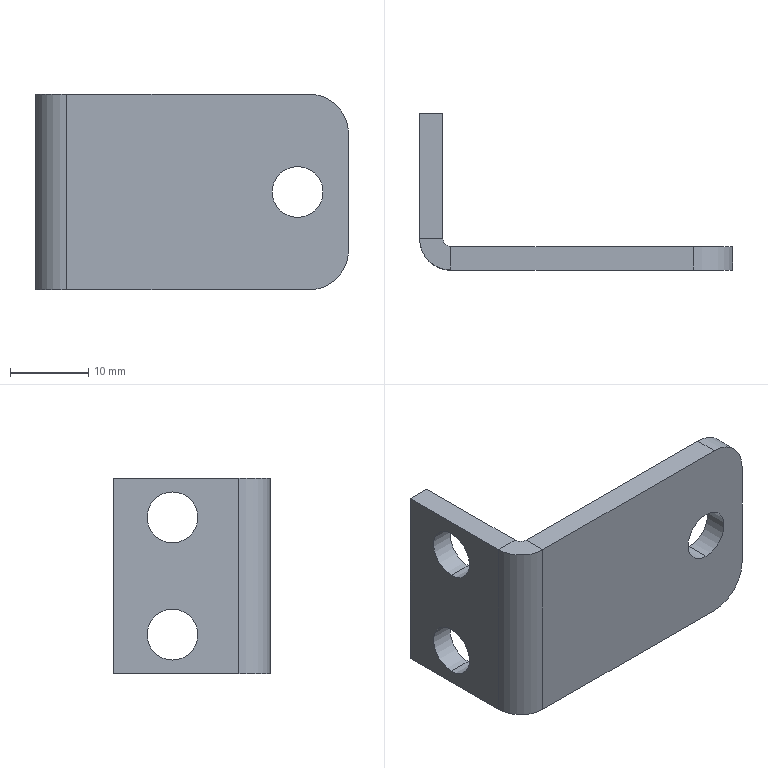Part | STEP file | Roller hanger plate | 1 solid | 22 faces | box 40 x 20 x 25 mm | volume 3864 mm3 | plane 12 | cylinder 10 | commonest cylinder face diameters 6.5 x6 10 x2 2 x1 8 x1
STEP:
#1=CARTESIAN_POINT('',(0.,0.,0.));
#2=DIRECTION('',(0.,0.,1.));
#3=DIRECTION('',(1.,0.,0.));
#4=AXIS2_PLACEMENT_3D('',#1,#2,#3);
#5=CARTESIAN_POINT('',(0.,12.5,4.25));
#6=VERTEX_POINT('',#5);
#7=CARTESIAN_POINT('',(3.,12.5,4.25));
#8=VERTEX_POINT('',#7);
#9=CARTESIAN_POINT('',(3.,12.5,4.25));
#10=DIRECTION('',(1.,0.,0.));
#11=VECTOR('',#10,1.);
#12=LINE('',#9,#11);
#13=CARTESIAN_POINT('',(3.,12.5,7.5));
#14=DIRECTION('',(1.,0.,0.));
#15=DIRECTION('',(0.,0.,-1.));
#16=AXIS2_PLACEMENT_3D('',#13,#14,#15);
#17=CYLINDRICAL_SURFACE('',#16,3.25);
#18=CARTESIAN_POINT('',(6.283,0.));
#19=DIRECTION('',(0.,1.));
#20=VECTOR('',#19,1.);
#21=LINE('',#18,#20);
#22=(GEOMETRIC_REPRESENTATION_CONTEXT(2)PARAMETRIC_REPRESENTATION_CONTEXT()REPRESENTATION_CONTEXT('',''));
#23=DEFINITIONAL_REPRESENTATION('',(#21),#22);
#24=PCURVE('',#17,#23);
#25=CARTESIAN_POINT('',(3.,12.5,7.5));
#26=DIRECTION('',(1.,0.,0.));
#27=DIRECTION('',(0.,0.,-1.));
#28=AXIS2_PLACEMENT_3D('',#25,#26,#27);
#29=CYLINDRICAL_SURFACE('',#28,3.25);
#30=CARTESIAN_POINT('',(0.,0.));
#31=DIRECTION('',(0.,1.));
#32=VECTOR('',#31,1.);
#33=LINE('',#30,#32);
#34=(GEOMETRIC_REPRESENTATION_CONTEXT(2)PARAMETRIC_REPRESENTATION_CONTEXT()REPRESENTATION_CONTEXT('',''));
#35=DEFINITIONAL_REPRESENTATION('',(#33),#34);
#36=PCURVE('',#29,#35);
#37=SURFACE_CURVE('',#12,(#24,#36),.PCURVE_S1.);
#38=EDGE_CURVE('',#6,#8,#37,.T.);
#39=ORIENTED_EDGE('',*,*,#38,.T.);
#40=CARTESIAN_POINT('',(3.,12.5,10.75));
#41=VERTEX_POINT('',#40);
#42=CARTESIAN_POINT('',(3.,12.5,7.5));
#43=DIRECTION('',(1.,0.,0.));
#44=DIRECTION('',(0.,0.,-1.));
#45=AXIS2_PLACEMENT_3D('',#42,#43,#44);
#46=CIRCLE('',#45,3.25);
#47=CARTESIAN_POINT('',(0.,0.));
#48=DIRECTION('',(1.,0.));
#49=VECTOR('',#48,1.);
#50=LINE('',#47,#49);
#51=(GEOMETRIC_REPRESENTATION_CONTEXT(2)PARAMETRIC_REPRESENTATION_CONTEXT()REPRESENTATION_CONTEXT('',''));
#52=DEFINITIONAL_REPRESENTATION('',(#50),#51);
#53=PCURVE('',#17,#52);
#54=CARTESIAN_POINT('',(3.,0.,12.5));
#55=DIRECTION('',(1.,0.,0.));
#56=DIRECTION('',(0.,0.,-1.));
#57=AXIS2_PLACEMENT_3D('',#54,#55,#56);
#58=PLANE('',#57);
#59=CARTESIAN_POINT('',(5.,12.5));
#60=DIRECTION('',(1.,0.));
#61=AXIS2_PLACEMENT_2D('',#59,#60);
#62=CIRCLE('',#61,3.25);
#63=(GEOMETRIC_REPRESENTATION_CONTEXT(2)PARAMETRIC_REPRESENTATION_CONTEXT()REPRESENTATION_CONTEXT('',''));
#64=DEFINITIONAL_REPRESENTATION('',(#62),#63);
#65=PCURVE('',#58,#64);
#66=SURFACE_CURVE('',#46,(#53,#65),.PCURVE_S1.);
#67=EDGE_CURVE('',#41,#8,#66,.T.);
#68=ORIENTED_EDGE('',*,*,#67,.F.);
#69=CARTESIAN_POINT('',(0.,12.5,10.75));
#70=VERTEX_POINT('',#69);
#71=CARTESIAN_POINT('',(3.,12.5,10.75));
#72=DIRECTION('',(1.,0.,0.));
#73=VECTOR('',#72,1.);
#74=LINE('',#71,#73);
#75=CARTESIAN_POINT('',(3.142,0.));
#76=DIRECTION('',(0.,1.));
#77=VECTOR('',#76,1.);
#78=LINE('',#75,#77);
#79=(GEOMETRIC_REPRESENTATION_CONTEXT(2)PARAMETRIC_REPRESENTATION_CONTEXT()REPRESENTATION_CONTEXT('',''));
#80=DEFINITIONAL_REPRESENTATION('',(#78),#79);
#81=PCURVE('',#17,#80);
#82=CARTESIAN_POINT('',(3.142,0.));
#83=DIRECTION('',(0.,1.));
#84=VECTOR('',#83,1.);
#85=LINE('',#82,#84);
#86=(GEOMETRIC_REPRESENTATION_CONTEXT(2)PARAMETRIC_REPRESENTATION_CONTEXT()REPRESENTATION_CONTEXT('',''));
#87=DEFINITIONAL_REPRESENTATION('',(#85),#86);
#88=PCURVE('',#29,#87);
#89=SURFACE_CURVE('',#74,(#81,#88),.PCURVE_S1.);
#90=EDGE_CURVE('',#70,#41,#89,.T.);
#91=ORIENTED_EDGE('',*,*,#90,.F.);
#92=CARTESIAN_POINT('',(0.,12.5,7.5));
#93=DIRECTION('',(1.,0.,0.));
#94=DIRECTION('',(0.,0.,-1.));
#95=AXIS2_PLACEMENT_3D('',#92,#93,#94);
#96=CIRCLE('',#95,3.25);
#97=CARTESIAN_POINT('',(0.,-3.));
#98=DIRECTION('',(1.,0.));
#99=VECTOR('',#98,1.);
#100=LINE('',#97,#99);
#101=(GEOMETRIC_REPRESENTATION_CONTEXT(2)PARAMETRIC_REPRESENTATION_CONTEXT()REPRESENTATION_CONTEXT('',''));
#102=DEFINITIONAL_REPRESENTATION('',(#100),#101);
#103=PCURVE('',#17,#102);
#104=CARTESIAN_POINT('',(0.,0.,12.5));
#105=DIRECTION('',(1.,0.,0.));
#106=DIRECTION('',(0.,0.,-1.));
#107=AXIS2_PLACEMENT_3D('',#104,#105,#106);
#108=PLANE('',#107);
#109=CARTESIAN_POINT('',(5.,12.5));
#110=DIRECTION('',(1.,0.));
#111=AXIS2_PLACEMENT_2D('',#109,#110);
#112=CIRCLE('',#111,3.25);
#113=(GEOMETRIC_REPRESENTATION_CONTEXT(2)PARAMETRIC_REPRESENTATION_CONTEXT()REPRESENTATION_CONTEXT('',''));
#114=DEFINITIONAL_REPRESENTATION('',(#112),#113);
#115=PCURVE('',#108,#114);
#116=SURFACE_CURVE('',#96,(#103,#115),.PCURVE_S1.);
#117=EDGE_CURVE('',#70,#6,#116,.T.);
#118=ORIENTED_EDGE('',*,*,#117,.T.);
#119=EDGE_LOOP('',(#39,#68,#91,#118));
#120=FACE_BOUND('',#119,.F.);
#121=ADVANCED_FACE('',(#120),#17,.F.);
#122=CARTESIAN_POINT('',(0.,12.5,-10.75));
#123=VERTEX_POINT('',#122);
#124=CARTESIAN_POINT('',(3.,12.5,-10.75));
#125=VERTEX_POINT('',#124);
#126=CARTESIAN_POINT('',(3.,12.5,-10.75));
#127=DIRECTION('',(1.,0.,0.));
#128=VECTOR('',#127,1.);
#129=LINE('',#126,#128);
#130=CARTESIAN_POINT('',(3.,12.5,-7.5));
#131=DIRECTION('',(1.,0.,0.));
#132=DIRECTION('',(0.,0.,-1.));
#133=AXIS2_PLACEMENT_3D('',#130,#131,#132);
#134=CYLINDRICAL_SURFACE('',#133,3.25);
#135=CARTESIAN_POINT('',(6.283,0.));
#136=DIRECTION('',(0.,1.));
#137=VECTOR('',#136,1.);
#138=LINE('',#135,#137);
#139=(GEOMETRIC_REPRESENTATION_CONTEXT(2)PARAMETRIC_REPRESENTATION_CONTEXT()REPRESENTATION_CONTEXT('',''));
#140=DEFINITIONAL_REPRESENTATION('',(#138),#139);
#141=PCURVE('',#134,#140);
#142=CARTESIAN_POINT('',(3.,12.5,-7.5));
#143=DIRECTION('',(1.,0.,0.));
#144=DIRECTION('',(0.,0.,-1.));
#145=AXIS2_PLACEMENT_3D('',#142,#143,#144);
#146=CYLINDRICAL_SURFACE('',#145,3.25);
#147=CARTESIAN_POINT('',(0.,0.));
#148=DIRECTION('',(0.,1.));
#149=VECTOR('',#148,1.);
#150=LINE('',#147,#149);
#151=(GEOMETRIC_REPRESENTATION_CONTEXT(2)PARAMETRIC_REPRESENTATION_CONTEXT()REPRESENTATION_CONTEXT('',''));
#152=DEFINITIONAL_REPRESENTATION('',(#150),#151);
#153=PCURVE('',#146,#152);
#154=SURFACE_CURVE('',#129,(#141,#153),.PCURVE_S1.);
#155=EDGE_CURVE('',#123,#125,#154,.T.);
#156=ORIENTED_EDGE('',*,*,#155,.T.);
#157=CARTESIAN_POINT('',(3.,12.5,-4.25));
#158=VERTEX_POINT('',#157);
#159=CARTESIAN_POINT('',(3.,12.5,-7.5));
#160=DIRECTION('',(1.,0.,0.));
#161=DIRECTION('',(0.,0.,-1.));
#162=AXIS2_PLACEMENT_3D('',#159,#160,#161);
#163=CIRCLE('',#162,3.25);
#164=CARTESIAN_POINT('',(0.,0.));
#165=DIRECTION('',(1.,0.));
#166=VECTOR('',#165,1.);
#167=LINE('',#164,#166);
#168=(GEOMETRIC_REPRESENTATION_CONTEXT(2)PARAMETRIC_REPRESENTATION_CONTEXT()REPRESENTATION_CONTEXT('',''));
#169=DEFINITIONAL_REPRESENTATION('',(#167),#168);
#170=PCURVE('',#134,#169);
#171=CARTESIAN_POINT('',(20.,12.5));
#172=DIRECTION('',(1.,0.));
#173=AXIS2_PLACEMENT_2D('',#171,#172);
#174=CIRCLE('',#173,3.25);
#175=(GEOMETRIC_REPRESENTATION_CONTEXT(2)PARAMETRIC_REPRESENTATION_CONTEXT()REPRESENTATION_CONTEXT('',''));
#176=DEFINITIONAL_REPRESENTATION('',(#174),#175);
#177=PCURVE('',#58,#176);
#178=SURFACE_CURVE('',#163,(#170,#177),.PCURVE_S1.);
#179=EDGE_CURVE('',#158,#125,#178,.T.);
#180=ORIENTED_EDGE('',*,*,#179,.F.);
#181=CARTESIAN_POINT('',(0.,12.5,-4.25));
#182=VERTEX_POINT('',#181);
#183=CARTESIAN_POINT('',(3.,12.5,-4.25));
#184=DIRECTION('',(1.,0.,0.));
#185=VECTOR('',#184,1.);
#186=LINE('',#183,#185);
#187=CARTESIAN_POINT('',(3.142,0.));
#188=DIRECTION('',(0.,1.));
#189=VECTOR('',#188,1.);
#190=LINE('',#187,#189);
#191=(GEOMETRIC_REPRESENTATION_CONTEXT(2)PARAMETRIC_REPRESENTATION_CONTEXT()REPRESENTATION_CONTEXT('',''));
#192=DEFINITIONAL_REPRESENTATION('',(#190),#191);
#193=PCURVE('',#134,#192);
#194=CARTESIAN_POINT('',(3.142,0.));
#195=DIRECTION('',(0.,1.));
#196=VECTOR('',#195,1.);
#197=LINE('',#194,#196);
#198=(GEOMETRIC_REPRESENTATION_CONTEXT(2)PARAMETRIC_REPRESENTATION_CONTEXT()REPRESENTATION_CONTEXT('',''));
#199=DEFINITIONAL_REPRESENTATION('',(#197),#198);
#200=PCURVE('',#146,#199);
#201=SURFACE_CURVE('',#186,(#193,#200),.PCURVE_S1.);
#202=EDGE_CURVE('',#182,#158,#201,.T.);
#203=ORIENTED_EDGE('',*,*,#202,.F.);
#204=CARTESIAN_POINT('',(0.,12.5,-7.5));
#205=DIRECTION('',(1.,0.,0.));
#206=DIRECTION('',(0.,0.,-1.));
#207=AXIS2_PLACEMENT_3D('',#204,#205,#206);
#208=CIRCLE('',#207,3.25);
#209=CARTESIAN_POINT('',(0.,-3.));
#210=DIRECTION('',(1.,0.));
#211=VECTOR('',#210,1.);
#212=LINE('',#209,#211);
#213=(GEOMETRIC_REPRESENTATION_CONTEXT(2)PARAMETRIC_REPRESENTATION_CONTEXT()REPRESENTATION_CONTEXT('',''));
#214=DEFINITIONAL_REPRESENTATION('',(#212),#213);
#215=PCURVE('',#134,#214);
#216=CARTESIAN_POINT('',(20.,12.5));
#217=DIRECTION('',(1.,0.));
#218=AXIS2_PLACEMENT_2D('',#216,#217);
#219=CIRCLE('',#218,3.25);
#220=(GEOMETRIC_REPRESENTATION_CONTEXT(2)PARAMETRIC_REPRESENTATION_CONTEXT()REPRESENTATION_CONTEXT('',''));
#221=DEFINITIONAL_REPRESENTATION('',(#219),#220);
#222=PCURVE('',#108,#221);
#223=SURFACE_CURVE('',#208,(#215,#222),.PCURVE_S1.);
#224=EDGE_CURVE('',#182,#123,#223,.T.);
#225=ORIENTED_EDGE('',*,*,#224,.T.);
#226=EDGE_LOOP('',(#156,#180,#203,#225));
#227=FACE_BOUND('',#226,.F.);
#228=ADVANCED_FACE('',(#227),#134,.F.);
#229=CARTESIAN_POINT('',(33.5,0.,3.25));
#230=VERTEX_POINT('',#229);
#231=CARTESIAN_POINT('',(33.5,3.,3.25));
#232=VERTEX_POINT('',#231);
#233=CARTESIAN_POINT('',(33.5,3.,3.25));
#234=DIRECTION('',(0.,1.,0.));
#235=VECTOR('',#234,1.);
#236=LINE('',#233,#235);
#237=CARTESIAN_POINT('',(33.5,3.,0.));
#238=DIRECTION('',(0.,1.,0.));
#239=DIRECTION('',(0.,0.,1.));
#240=AXIS2_PLACEMENT_3D('',#237,#238,#239);
#241=CYLINDRICAL_SURFACE('',#240,3.25);
#242=CARTESIAN_POINT('',(6.283,0.));
#243=DIRECTION('',(0.,1.));
#244=VECTOR('',#243,1.);
#245=LINE('',#242,#244);
#246=(GEOMETRIC_REPRESENTATION_CONTEXT(2)PARAMETRIC_REPRESENTATION_CONTEXT()REPRESENTATION_CONTEXT('',''));
#247=DEFINITIONAL_REPRESENTATION('',(#245),#246);
#248=PCURVE('',#241,#247);
#249=CARTESIAN_POINT('',(33.5,3.,0.));
#250=DIRECTION('',(0.,1.,0.));
#251=DIRECTION('',(0.,0.,1.));
#252=AXIS2_PLACEMENT_3D('',#249,#250,#251);
#253=CYLINDRICAL_SURFACE('',#252,3.25);
#254=CARTESIAN_POINT('',(0.,0.));
#255=DIRECTION('',(0.,1.));
#256=VECTOR('',#255,1.);
#257=LINE('',#254,#256);
#258=(GEOMETRIC_REPRESENTATION_CONTEXT(2)PARAMETRIC_REPRESENTATION_CONTEXT()REPRESENTATION_CONTEXT('',''));
#259=DEFINITIONAL_REPRESENTATION('',(#257),#258);
#260=PCURVE('',#253,#259);
#261=SURFACE_CURVE('',#236,(#248,#260),.PCURVE_S1.);
#262=EDGE_CURVE('',#230,#232,#261,.T.);
#263=ORIENTED_EDGE('',*,*,#262,.T.);
#264=CARTESIAN_POINT('',(33.5,3.,-3.25));
#265=VERTEX_POINT('',#264);
#266=CARTESIAN_POINT('',(33.5,3.,0.));
#267=DIRECTION('',(0.,1.,0.));
#268=DIRECTION('',(0.,0.,1.));
#269=AXIS2_PLACEMENT_3D('',#266,#267,#268);
#270=CIRCLE('',#269,3.25);
#271=CARTESIAN_POINT('',(0.,0.));
#272=DIRECTION('',(1.,0.));
#273=VECTOR('',#272,1.);
#274=LINE('',#271,#273);
#275=(GEOMETRIC_REPRESENTATION_CONTEXT(2)PARAMETRIC_REPRESENTATION_CONTEXT()REPRESENTATION_CONTEXT('',''));
#276=DEFINITIONAL_REPRESENTATION('',(#274),#275);
#277=PCURVE('',#241,#276);
#278=CARTESIAN_POINT('',(0.,3.,12.5));
#279=DIRECTION('',(0.,1.,0.));
#280=DIRECTION('',(0.,0.,1.));
#281=AXIS2_PLACEMENT_3D('',#278,#279,#280);
#282=PLANE('',#281);
#283=CARTESIAN_POINT('',(-12.5,33.5));
#284=DIRECTION('',(1.,0.));
#285=AXIS2_PLACEMENT_2D('',#283,#284);
#286=CIRCLE('',#285,3.25);
#287=(GEOMETRIC_REPRESENTATION_CONTEXT(2)PARAMETRIC_REPRESENTATION_CONTEXT()REPRESENTATION_CONTEXT('',''));
#288=DEFINITIONAL_REPRESENTATION('',(#286),#287);
#289=PCURVE('',#282,#288);
#290=SURFACE_CURVE('',#270,(#277,#289),.PCURVE_S1.);
#291=EDGE_CURVE('',#265,#232,#290,.T.);
#292=ORIENTED_EDGE('',*,*,#291,.F.);
#293=CARTESIAN_POINT('',(33.5,0.,-3.25));
#294=VERTEX_POINT('',#293);
#295=CARTESIAN_POINT('',(33.5,3.,-3.25));
#296=DIRECTION('',(0.,1.,0.));
#297=VECTOR('',#296,1.);
#298=LINE('',#295,#297);
#299=CARTESIAN_POINT('',(3.142,0.));
#300=DIRECTION('',(0.,1.));
#301=VECTOR('',#300,1.);
#302=LINE('',#299,#301);
#303=(GEOMETRIC_REPRESENTATION_CONTEXT(2)PARAMETRIC_REPRESENTATION_CONTEXT()REPRESENTATION_CONTEXT('',''));
#304=DEFINITIONAL_REPRESENTATION('',(#302),#303);
#305=PCURVE('',#241,#304);
#306=CARTESIAN_POINT('',(3.142,0.));
#307=DIRECTION('',(0.,1.));
#308=VECTOR('',#307,1.);
#309=LINE('',#306,#308);
#310=(GEOMETRIC_REPRESENTATION_CONTEXT(2)PARAMETRIC_REPRESENTATION_CONTEXT()REPRESENTATION_CONTEXT('',''));
#311=DEFINITIONAL_REPRESENTATION('',(#309),#310);
#312=PCURVE('',#253,#311);
#313=SURFACE_CURVE('',#298,(#305,#312),.PCURVE_S1.);
#314=EDGE_CURVE('',#294,#265,#313,.T.);
#315=ORIENTED_EDGE('',*,*,#314,.F.);
#316=CARTESIAN_POINT('',(33.5,0.,0.));
#317=DIRECTION('',(0.,1.,0.));
#318=DIRECTION('',(0.,0.,1.));
#319=AXIS2_PLACEMENT_3D('',#316,#317,#318);
#320=CIRCLE('',#319,3.25);
#321=CARTESIAN_POINT('',(0.,-3.));
#322=DIRECTION('',(1.,0.));
#323=VECTOR('',#322,1.);
#324=LINE('',#321,#323);
#325=(GEOMETRIC_REPRESENTATION_CONTEXT(2)PARAMETRIC_REPRESENTATION_CONTEXT()REPRESENTATION_CONTEXT('',''));
#326=DEFINITIONAL_REPRESENTATION('',(#324),#325);
#327=PCURVE('',#241,#326);
#328=CARTESIAN_POINT('',(0.,0.,12.5));
#329=DIRECTION('',(0.,1.,0.));
#330=DIRECTION('',(0.,0.,1.));
#331=AXIS2_PLACEMENT_3D('',#328,#329,#330);
#332=PLANE('',#331);
#333=CARTESIAN_POINT('',(-12.5,33.5));
#334=DIRECTION('',(1.,0.));
#335=AXIS2_PLACEMENT_2D('',#333,#334);
#336=CIRCLE('',#335,3.25);
#337=(GEOMETRIC_REPRESENTATION_CONTEXT(2)PARAMETRIC_REPRESENTATION_CONTEXT()REPRESENTATION_CONTEXT('',''));
#338=DEFINITIONAL_REPRESENTATION('',(#336),#337);
#339=PCURVE('',#332,#338);
#340=SURFACE_CURVE('',#320,(#327,#339),.PCURVE_S1.);
#341=EDGE_CURVE('',#294,#230,#340,.T.);
#342=ORIENTED_EDGE('',*,*,#341,.T.);
#343=EDGE_LOOP('',(#263,#292,#315,#342));
#344=FACE_BOUND('',#343,.F.);
#345=ADVANCED_FACE('',(#344),#241,.F.);
#346=CARTESIAN_POINT('',(0.,4.,12.5));
#347=VERTEX_POINT('',#346);
#348=CARTESIAN_POINT('',(3.,4.,12.5));
#349=VERTEX_POINT('',#348);
#350=CARTESIAN_POINT('',(0.,4.,12.5));
#351=DIRECTION('',(1.,0.,0.));
#352=VECTOR('',#351,1.);
#353=LINE('',#350,#352);
#354=CARTESIAN_POINT('',(0.,4.,12.5));
#355=DIRECTION('',(0.,0.,1.));
#356=DIRECTION('',(1.,0.,0.));
#357=AXIS2_PLACEMENT_3D('',#354,#355,#356);
#358=PLANE('',#357);
#359=CARTESIAN_POINT('',(0.,0.));
#360=DIRECTION('',(1.,0.));
#361=VECTOR('',#360,1.);
#362=LINE('',#359,#361);
#363=(GEOMETRIC_REPRESENTATION_CONTEXT(2)PARAMETRIC_REPRESENTATION_CONTEXT()REPRESENTATION_CONTEXT('',''));
#364=DEFINITIONAL_REPRESENTATION('',(#362),#363);
#365=PCURVE('',#358,#364);
#366=CARTESIAN_POINT('',(4.,3.,12.5));
#367=DIRECTION('',(0.,0.,1.));
#368=DIRECTION('',(1.,0.,0.));
#369=AXIS2_PLACEMENT_3D('',#366,#367,#368);
#370=PLANE('',#369);
#371=CARTESIAN_POINT('',(-4.,1.));
#372=DIRECTION('',(1.,0.));
#373=VECTOR('',#372,1.);
#374=LINE('',#371,#373);
#375=(GEOMETRIC_REPRESENTATION_CONTEXT(2)PARAMETRIC_REPRESENTATION_CONTEXT()REPRESENTATION_CONTEXT('',''));
#376=DEFINITIONAL_REPRESENTATION('',(#374),#375);
#377=PCURVE('',#370,#376);
#378=SURFACE_CURVE('',#353,(#365,#377),.PCURVE_S1.);
#379=EDGE_CURVE('',#347,#349,#378,.T.);
#380=ORIENTED_EDGE('',*,*,#379,.F.);
#381=CARTESIAN_POINT('',(4.,0.,12.5));
#382=VERTEX_POINT('',#381);
#383=CARTESIAN_POINT('',(4.,4.,12.5));
#384=DIRECTION('',(0.,0.,1.));
#385=DIRECTION('',(-1.,0.,0.));
#386=AXIS2_PLACEMENT_3D('',#383,#384,#385);
#387=CIRCLE('',#386,4.);
#388=CARTESIAN_POINT('',(4.,0.));
#389=DIRECTION('',(-1.,0.));
#390=AXIS2_PLACEMENT_2D('',#388,#389);
#391=CIRCLE('',#390,4.);
#392=(GEOMETRIC_REPRESENTATION_CONTEXT(2)PARAMETRIC_REPRESENTATION_CONTEXT()REPRESENTATION_CONTEXT('',''));
#393=DEFINITIONAL_REPRESENTATION('',(#391),#392);
#394=PCURVE('',#358,#393);
#395=CARTESIAN_POINT('',(4.,4.,12.5));
#396=DIRECTION('',(0.,0.,-1.));
#397=DIRECTION('',(-1.,0.,0.));
#398=AXIS2_PLACEMENT_3D('',#395,#396,#397);
#399=CYLINDRICAL_SURFACE('',#398,4.);
#400=CARTESIAN_POINT('',(6.283,0.));
#401=DIRECTION('',(-1.,0.));
#402=VECTOR('',#401,1.);
#403=LINE('',#400,#402);
#404=(GEOMETRIC_REPRESENTATION_CONTEXT(2)PARAMETRIC_REPRESENTATION_CONTEXT()REPRESENTATION_CONTEXT('',''));
#405=DEFINITIONAL_REPRESENTATION('',(#403),#404);
#406=PCURVE('',#399,#405);
#407=SURFACE_CURVE('',#387,(#394,#406),.PCURVE_S1.);
#408=EDGE_CURVE('',#347,#382,#407,.T.);
#409=ORIENTED_EDGE('',*,*,#408,.T.);
#410=CARTESIAN_POINT('',(4.,3.,12.5));
#411=VERTEX_POINT('',#410);
#412=CARTESIAN_POINT('',(4.,3.,12.5));
#413=DIRECTION('',(0.,-1.,0.));
#414=VECTOR('',#413,1.);
#415=LINE('',#412,#414);
#416=CARTESIAN_POINT('',(4.,-1.));
#417=DIRECTION('',(0.,-1.));
#418=VECTOR('',#417,1.);
#419=LINE('',#416,#418);
#420=(GEOMETRIC_REPRESENTATION_CONTEXT(2)PARAMETRIC_REPRESENTATION_CONTEXT()REPRESENTATION_CONTEXT('',''));
#421=DEFINITIONAL_REPRESENTATION('',(#419),#420);
#422=PCURVE('',#358,#421);
#423=CARTESIAN_POINT('',(4.,4.,12.5));
#424=DIRECTION('',(0.,0.,1.));
#425=DIRECTION('',(1.,0.,0.));
#426=AXIS2_PLACEMENT_3D('',#423,#424,#425);
#427=PLANE('',#426);
#428=CARTESIAN_POINT('',(0.,-1.));
#429=DIRECTION('',(0.,-1.));
#430=VECTOR('',#429,1.);
#431=LINE('',#428,#430);
#432=(GEOMETRIC_REPRESENTATION_CONTEXT(2)PARAMETRIC_REPRESENTATION_CONTEXT()REPRESENTATION_CONTEXT('',''));
#433=DEFINITIONAL_REPRESENTATION('',(#431),#432);
#434=PCURVE('',#427,#433);
#435=SURFACE_CURVE('',#415,(#422,#434),.PCURVE_S1.);
#436=EDGE_CURVE('',#411,#382,#435,.T.);
#437=ORIENTED_EDGE('',*,*,#436,.F.);
#438=CARTESIAN_POINT('',(4.,4.,12.5));
#439=DIRECTION('',(0.,0.,1.));
#440=DIRECTION('',(1.,0.,0.));
#441=AXIS2_PLACEMENT_3D('',#438,#439,#440);
#442=CIRCLE('',#441,1.);
#443=CARTESIAN_POINT('',(4.,0.));
#444=DIRECTION('',(1.,0.));
#445=AXIS2_PLACEMENT_2D('',#443,#444);
#446=CIRCLE('',#445,1.);
#447=(GEOMETRIC_REPRESENTATION_CONTEXT(2)PARAMETRIC_REPRESENTATION_CONTEXT()REPRESENTATION_CONTEXT('',''));
#448=DEFINITIONAL_REPRESENTATION('',(#446),#447);
#449=PCURVE('',#358,#448);
#450=CARTESIAN_POINT('',(4.,4.,12.5));
#451=DIRECTION('',(0.,0.,-1.));
#452=DIRECTION('',(-1.,0.,0.));
#453=AXIS2_PLACEMENT_3D('',#450,#451,#452);
#454=CYLINDRICAL_SURFACE('',#453,1.);
#455=CARTESIAN_POINT('',(9.425,0.));
#456=DIRECTION('',(-1.,0.));
#457=VECTOR('',#456,1.);
#458=LINE('',#455,#457);
#459=(GEOMETRIC_REPRESENTATION_CONTEXT(2)PARAMETRIC_REPRESENTATION_CONTEXT()REPRESENTATION_CONTEXT('',''));
#460=DEFINITIONAL_REPRESENTATION('',(#458),#459);
#461=PCURVE('',#454,#460);
#462=SURFACE_CURVE('',#442,(#449,#461),.PCURVE_S1.);
#463=EDGE_CURVE('',#349,#411,#462,.T.);
#464=ORIENTED_EDGE('',*,*,#463,.F.);
#465=EDGE_LOOP('',(#380,#409,#437,#464));
#466=FACE_BOUND('',#465,.T.);
#467=ADVANCED_FACE('',(#466),#358,.T.);
#468=CARTESIAN_POINT('',(0.,20.,12.5));
#469=VERTEX_POINT('',#468);
#470=CARTESIAN_POINT('',(0.,0.,12.5));
#471=DIRECTION('',(0.,-1.,0.));
#472=VECTOR('',#471,1.);
#473=LINE('',#470,#472);
#474=CARTESIAN_POINT('',(-4.,-3.));
#475=DIRECTION('',(0.,-1.));
#476=VECTOR('',#475,1.);
#477=LINE('',#474,#476);
#478=(GEOMETRIC_REPRESENTATION_CONTEXT(2)PARAMETRIC_REPRESENTATION_CONTEXT()REPRESENTATION_CONTEXT('',''));
#479=DEFINITIONAL_REPRESENTATION('',(#477),#478);
#480=PCURVE('',#370,#479);
#481=CARTESIAN_POINT('',(0.,0.));
#482=DIRECTION('',(0.,-1.));
#483=VECTOR('',#482,1.);
#484=LINE('',#481,#483);
#485=(GEOMETRIC_REPRESENTATION_CONTEXT(2)PARAMETRIC_REPRESENTATION_CONTEXT()REPRESENTATION_CONTEXT('',''));
#486=DEFINITIONAL_REPRESENTATION('',(#484),#485);
#487=PCURVE('',#108,#486);
#488=SURFACE_CURVE('',#473,(#480,#487),.PCURVE_S1.);
#489=EDGE_CURVE('',#469,#347,#488,.T.);
#490=ORIENTED_EDGE('',*,*,#489,.T.);
#491=ORIENTED_EDGE('',*,*,#379,.T.);
#492=CARTESIAN_POINT('',(3.,20.,12.5));
#493=VERTEX_POINT('',#492);
#494=CARTESIAN_POINT('',(3.,0.,12.5));
#495=DIRECTION('',(0.,-1.,0.));
#496=VECTOR('',#495,1.);
#497=LINE('',#494,#496);
#498=CARTESIAN_POINT('',(-1.,-3.));
#499=DIRECTION('',(0.,-1.));
#500=VECTOR('',#499,1.);
#501=LINE('',#498,#500);
#502=(GEOMETRIC_REPRESENTATION_CONTEXT(2)PARAMETRIC_REPRESENTATION_CONTEXT()REPRESENTATION_CONTEXT('',''));
#503=DEFINITIONAL_REPRESENTATION('',(#501),#502);
#504=PCURVE('',#370,#503);
#505=CARTESIAN_POINT('',(0.,0.));
#506=DIRECTION('',(0.,-1.));
#507=VECTOR('',#506,1.);
#508=LINE('',#505,#507);
#509=(GEOMETRIC_REPRESENTATION_CONTEXT(2)PARAMETRIC_REPRESENTATION_CONTEXT()REPRESENTATION_CONTEXT('',''));
#510=DEFINITIONAL_REPRESENTATION('',(#508),#509);
#511=PCURVE('',#58,#510);
#512=SURFACE_CURVE('',#497,(#504,#511),.PCURVE_S1.);
#513=EDGE_CURVE('',#493,#349,#512,.T.);
#514=ORIENTED_EDGE('',*,*,#513,.F.);
#515=CARTESIAN_POINT('',(0.,20.,12.5));
#516=DIRECTION('',(1.,0.,0.));
#517=VECTOR('',#516,1.);
#518=LINE('',#515,#517);
#519=CARTESIAN_POINT('',(-4.,17.));
#520=DIRECTION('',(1.,0.));
#521=VECTOR('',#520,1.);
#522=LINE('',#519,#521);
#523=(GEOMETRIC_REPRESENTATION_CONTEXT(2)PARAMETRIC_REPRESENTATION_CONTEXT()REPRESENTATION_CONTEXT('',''));
#524=DEFINITIONAL_REPRESENTATION('',(#522),#523);
#525=PCURVE('',#370,#524);
#526=CARTESIAN_POINT('',(0.,20.,12.5));
#527=DIRECTION('',(0.,1.,0.));
#528=DIRECTION('',(0.,0.,1.));
#529=AXIS2_PLACEMENT_3D('',#526,#527,#528);
#530=PLANE('',#529);
#531=CARTESIAN_POINT('',(0.,0.));
#532=DIRECTION('',(0.,1.));
#533=VECTOR('',#532,1.);
#534=LINE('',#531,#533);
#535=(GEOMETRIC_REPRESENTATION_CONTEXT(2)PARAMETRIC_REPRESENTATION_CONTEXT()REPRESENTATION_CONTEXT('',''));
#536=DEFINITIONAL_REPRESENTATION('',(#534),#535);
#537=PCURVE('',#530,#536);
#538=SURFACE_CURVE('',#518,(#525,#537),.PCURVE_S1.);
#539=EDGE_CURVE('',#469,#493,#538,.T.);
#540=ORIENTED_EDGE('',*,*,#539,.F.);
#541=EDGE_LOOP('',(#490,#491,#514,#540));
#542=FACE_BOUND('',#541,.T.);
#543=ADVANCED_FACE('',(#542),#370,.T.);
#544=CARTESIAN_POINT('',(4.,0.,-12.5));
#545=VERTEX_POINT('',#544);
#546=CARTESIAN_POINT('',(4.,3.,-12.5));
#547=VERTEX_POINT('',#546);
#548=CARTESIAN_POINT('',(4.,0.,-12.5));
#549=DIRECTION('',(0.,1.,0.));
#550=VECTOR('',#549,1.);
#551=LINE('',#548,#550);
#552=CARTESIAN_POINT('',(4.,0.,-12.5));
#553=DIRECTION('',(0.,0.,-1.));
#554=DIRECTION('',(-1.,0.,0.));
#555=AXIS2_PLACEMENT_3D('',#552,#553,#554);
#556=PLANE('',#555);
#557=CARTESIAN_POINT('',(0.,0.));
#558=DIRECTION('',(0.,1.));
#559=VECTOR('',#558,1.);
#560=LINE('',#557,#559);
#561=(GEOMETRIC_REPRESENTATION_CONTEXT(2)PARAMETRIC_REPRESENTATION_CONTEXT()REPRESENTATION_CONTEXT('',''));
#562=DEFINITIONAL_REPRESENTATION('',(#560),#561);
#563=PCURVE('',#556,#562);
#564=CARTESIAN_POINT('',(3.,4.,-12.5));
#565=DIRECTION('',(0.,0.,-1.));
#566=DIRECTION('',(-1.,0.,0.));
#567=AXIS2_PLACEMENT_3D('',#564,#565,#566);
#568=PLANE('',#567);
#569=CARTESIAN_POINT('',(-1.,-4.));
#570=DIRECTION('',(0.,1.));
#571=VECTOR('',#570,1.);
#572=LINE('',#569,#571);
#573=(GEOMETRIC_REPRESENTATION_CONTEXT(2)PARAMETRIC_REPRESENTATION_CONTEXT()REPRESENTATION_CONTEXT('',''));
#574=DEFINITIONAL_REPRESENTATION('',(#572),#573);
#575=PCURVE('',#568,#574);
#576=SURFACE_CURVE('',#551,(#563,#575),.PCURVE_S1.);
#577=EDGE_CURVE('',#545,#547,#576,.T.);
#578=ORIENTED_EDGE('',*,*,#577,.F.);
#579=CARTESIAN_POINT('',(0.,4.,-12.5));
#580=VERTEX_POINT('',#579);
#581=CARTESIAN_POINT('',(4.,4.,-12.5));
#582=DIRECTION('',(0.,0.,1.));
#583=DIRECTION('',(-1.,0.,0.));
#584=AXIS2_PLACEMENT_3D('',#581,#582,#583);
#585=CIRCLE('',#584,4.);
#586=CARTESIAN_POINT('',(4.,4.));
#587=CARTESIAN_POINT('',(4.,-2.928));
#588=CARTESIAN_POINT('',(-2.,0.5359));
#589=CARTESIAN_POINT('',(-8.,4.));
#590=CARTESIAN_POINT('',(-2.,7.464));
#591=CARTESIAN_POINT('',(4.,10.928));
#592=CARTESIAN_POINT('',(4.,4.));
#593=(BOUNDED_CURVE()B_SPLINE_CURVE(2,(#586,#587,#588,#589,#590,#591,#592),.UNSPECIFIED.,.T.,.F.)B_SPLINE_CURVE_WITH_KNOTS((1,2,2,2,2,1),(-2.094,0.,2.094,4.189,6.283,8.378),.UNSPECIFIED.)CURVE()GEOMETRIC_REPRESENTATION_ITEM()RATIONAL_B_SPLINE_CURVE((1.,0.5,1.,0.5,1.,0.5,1.))REPRESENTATION_ITEM(''));
#594=(GEOMETRIC_REPRESENTATION_CONTEXT(2)PARAMETRIC_REPRESENTATION_CONTEXT()REPRESENTATION_CONTEXT('',''));
#595=DEFINITIONAL_REPRESENTATION('',(#593),#594);
#596=PCURVE('',#556,#595);
#597=CARTESIAN_POINT('',(6.283,25.));
#598=DIRECTION('',(-1.,0.));
#599=VECTOR('',#598,1.);
#600=LINE('',#597,#599);
#601=(GEOMETRIC_REPRESENTATION_CONTEXT(2)PARAMETRIC_REPRESENTATION_CONTEXT()REPRESENTATION_CONTEXT('',''));
#602=DEFINITIONAL_REPRESENTATION('',(#600),#601);
#603=PCURVE('',#399,#602);
#604=SURFACE_CURVE('',#585,(#596,#603),.PCURVE_S1.);
#605=EDGE_CURVE('',#580,#545,#604,.T.);
#606=ORIENTED_EDGE('',*,*,#605,.F.);
#607=CARTESIAN_POINT('',(3.,4.,-12.5));
#608=VERTEX_POINT('',#607);
#609=CARTESIAN_POINT('',(3.,4.,-12.5));
#610=DIRECTION('',(-1.,0.,0.));
#611=VECTOR('',#610,1.);
#612=LINE('',#609,#611);
#613=CARTESIAN_POINT('',(1.,4.));
#614=DIRECTION('',(1.,0.));
#615=VECTOR('',#614,1.);
#616=LINE('',#613,#615);
#617=(GEOMETRIC_REPRESENTATION_CONTEXT(2)PARAMETRIC_REPRESENTATION_CONTEXT()REPRESENTATION_CONTEXT('',''));
#618=DEFINITIONAL_REPRESENTATION('',(#616),#617);
#619=PCURVE('',#556,#618);
#620=CARTESIAN_POINT('',(4.,4.,-12.5));
#621=DIRECTION('',(0.,0.,1.));
#622=DIRECTION('',(1.,0.,0.));
#623=AXIS2_PLACEMENT_3D('',#620,#621,#622);
#624=PLANE('',#623);
#625=CARTESIAN_POINT('',(-1.,0.));
#626=DIRECTION('',(-1.,0.));
#627=VECTOR('',#626,1.);
#628=LINE('',#625,#627);
#629=(GEOMETRIC_REPRESENTATION_CONTEXT(2)PARAMETRIC_REPRESENTATION_CONTEXT()REPRESENTATION_CONTEXT('',''));
#630=DEFINITIONAL_REPRESENTATION('',(#628),#629);
#631=PCURVE('',#624,#630);
#632=SURFACE_CURVE('',#612,(#619,#631),.PCURVE_S1.);
#633=EDGE_CURVE('',#608,#580,#632,.T.);
#634=ORIENTED_EDGE('',*,*,#633,.F.);
#635=CARTESIAN_POINT('',(4.,4.,-12.5));
#636=DIRECTION('',(0.,0.,1.));
#637=DIRECTION('',(1.,0.,0.));
#638=AXIS2_PLACEMENT_3D('',#635,#636,#637);
#639=CIRCLE('',#638,1.);
#640=CARTESIAN_POINT('',(-1.,4.));
#641=CARTESIAN_POINT('',(-1.,5.732));
#642=CARTESIAN_POINT('',(0.5,4.866));
#643=CARTESIAN_POINT('',(2.,4.));
#644=CARTESIAN_POINT('',(0.5,3.134));
#645=CARTESIAN_POINT('',(-1.,2.268));
#646=CARTESIAN_POINT('',(-1.,4.));
#647=(BOUNDED_CURVE()B_SPLINE_CURVE(2,(#640,#641,#642,#643,#644,#645,#646),.UNSPECIFIED.,.T.,.F.)B_SPLINE_CURVE_WITH_KNOTS((1,2,2,2,2,1),(-2.094,0.,2.094,4.189,6.283,8.378),.UNSPECIFIED.)CURVE()GEOMETRIC_REPRESENTATION_ITEM()RATIONAL_B_SPLINE_CURVE((1.,0.5,1.,0.5,1.,0.5,1.))REPRESENTATION_ITEM(''));
#648=(GEOMETRIC_REPRESENTATION_CONTEXT(2)PARAMETRIC_REPRESENTATION_CONTEXT()REPRESENTATION_CONTEXT('',''));
#649=DEFINITIONAL_REPRESENTATION('',(#647),#648);
#650=PCURVE('',#556,#649);
#651=CARTESIAN_POINT('',(9.425,25.));
#652=DIRECTION('',(-1.,0.));
#653=VECTOR('',#652,1.);
#654=LINE('',#651,#653);
#655=(GEOMETRIC_REPRESENTATION_CONTEXT(2)PARAMETRIC_REPRESENTATION_CONTEXT()REPRESENTATION_CONTEXT('',''));
#656=DEFINITIONAL_REPRESENTATION('',(#654),#655);
#657=PCURVE('',#454,#656);
#658=SURFACE_CURVE('',#639,(#650,#657),.PCURVE_S1.);
#659=EDGE_CURVE('',#608,#547,#658,.T.);
#660=ORIENTED_EDGE('',*,*,#659,.T.);
#661=EDGE_LOOP('',(#578,#606,#634,#660));
#662=FACE_BOUND('',#661,.T.);
#663=ADVANCED_FACE('',(#662),#556,.T.);
#664=CARTESIAN_POINT('',(35.,3.,-12.5));
#665=VERTEX_POINT('',#664);
#666=CARTESIAN_POINT('',(0.,3.,-12.5));
#667=DIRECTION('',(1.,0.,0.));
#668=VECTOR('',#667,1.);
#669=LINE('',#666,#668);
#670=CARTESIAN_POINT('',(3.,-1.));
#671=DIRECTION('',(-1.,0.));
#672=VECTOR('',#671,1.);
#673=LINE('',#670,#672);
#674=(GEOMETRIC_REPRESENTATION_CONTEXT(2)PARAMETRIC_REPRESENTATION_CONTEXT()REPRESENTATION_CONTEXT('',''));
#675=DEFINITIONAL_REPRESENTATION('',(#673),#674);
#676=PCURVE('',#568,#675);
#677=CARTESIAN_POINT('',(-25.,0.));
#678=DIRECTION('',(0.,1.));
#679=VECTOR('',#678,1.);
#680=LINE('',#677,#679);
#681=(GEOMETRIC_REPRESENTATION_CONTEXT(2)PARAMETRIC_REPRESENTATION_CONTEXT()REPRESENTATION_CONTEXT('',''));
#682=DEFINITIONAL_REPRESENTATION('',(#680),#681);
#683=PCURVE('',#282,#682);
#684=SURFACE_CURVE('',#669,(#676,#683),.PCURVE_S1.);
#685=EDGE_CURVE('',#547,#665,#684,.T.);
#686=ORIENTED_EDGE('',*,*,#685,.T.);
#687=CARTESIAN_POINT('',(35.,0.,-12.5));
#688=VERTEX_POINT('',#687);
#689=CARTESIAN_POINT('',(35.,4.,-12.5));
#690=DIRECTION('',(0.,-1.,0.));
#691=VECTOR('',#690,1.);
#692=LINE('',#689,#691);
#693=CARTESIAN_POINT('',(-32.,0.));
#694=DIRECTION('',(0.,-1.));
#695=VECTOR('',#694,1.);
#696=LINE('',#693,#695);
#697=(GEOMETRIC_REPRESENTATION_CONTEXT(2)PARAMETRIC_REPRESENTATION_CONTEXT()REPRESENTATION_CONTEXT('',''));
#698=DEFINITIONAL_REPRESENTATION('',(#696),#697);
#699=PCURVE('',#568,#698);
#700=CARTESIAN_POINT('',(35.,4.,-7.5));
#701=DIRECTION('',(0.,-1.,0.));
#702=DIRECTION('',(0.,0.,-1.));
#703=AXIS2_PLACEMENT_3D('',#700,#701,#702);
#704=CYLINDRICAL_SURFACE('',#703,5.);
#705=CARTESIAN_POINT('',(0.,0.));
#706=DIRECTION('',(0.,1.));
#707=VECTOR('',#706,1.);
#708=LINE('',#705,#707);
#709=(GEOMETRIC_REPRESENTATION_CONTEXT(2)PARAMETRIC_REPRESENTATION_CONTEXT()REPRESENTATION_CONTEXT('',''));
#710=DEFINITIONAL_REPRESENTATION('',(#708),#709);
#711=PCURVE('',#704,#710);
#712=SURFACE_CURVE('',#692,(#699,#711),.PCURVE_S1.);
#713=EDGE_CURVE('',#665,#688,#712,.T.);
#714=ORIENTED_EDGE('',*,*,#713,.T.);
#715=CARTESIAN_POINT('',(0.,0.,-12.5));
#716=DIRECTION('',(1.,0.,0.));
#717=VECTOR('',#716,1.);
#718=LINE('',#715,#717);
#719=CARTESIAN_POINT('',(3.,-4.));
#720=DIRECTION('',(-1.,0.));
#721=VECTOR('',#720,1.);
#722=LINE('',#719,#721);
#723=(GEOMETRIC_REPRESENTATION_CONTEXT(2)PARAMETRIC_REPRESENTATION_CONTEXT()REPRESENTATION_CONTEXT('',''));
#724=DEFINITIONAL_REPRESENTATION('',(#722),#723);
#725=PCURVE('',#568,#724);
#726=CARTESIAN_POINT('',(-25.,0.));
#727=DIRECTION('',(0.,1.));
#728=VECTOR('',#727,1.);
#729=LINE('',#726,#728);
#730=(GEOMETRIC_REPRESENTATION_CONTEXT(2)PARAMETRIC_REPRESENTATION_CONTEXT()REPRESENTATION_CONTEXT('',''));
#731=DEFINITIONAL_REPRESENTATION('',(#729),#730);
#732=PCURVE('',#332,#731);
#733=SURFACE_CURVE('',#718,(#725,#732),.PCURVE_S1.);
#734=EDGE_CURVE('',#545,#688,#733,.T.);
#735=ORIENTED_EDGE('',*,*,#734,.F.);
#736=ORIENTED_EDGE('',*,*,#577,.T.);
#737=EDGE_LOOP('',(#686,#714,#735,#736));
#738=FACE_BOUND('',#737,.T.);
#739=ADVANCED_FACE('',(#738),#568,.T.);
#740=CARTESIAN_POINT('',(33.5,0.,0.));
#741=DIRECTION('',(0.,1.,0.));
#742=DIRECTION('',(0.,0.,1.));
#743=AXIS2_PLACEMENT_3D('',#740,#741,#742);
#744=CIRCLE('',#743,3.25);
#745=CARTESIAN_POINT('',(-12.5,33.5));
#746=DIRECTION('',(1.,0.));
#747=AXIS2_PLACEMENT_2D('',#745,#746);
#748=CIRCLE('',#747,3.25);
#749=(GEOMETRIC_REPRESENTATION_CONTEXT(2)PARAMETRIC_REPRESENTATION_CONTEXT()REPRESENTATION_CONTEXT('',''));
#750=DEFINITIONAL_REPRESENTATION('',(#748),#749);
#751=PCURVE('',#332,#750);
#752=CARTESIAN_POINT('',(0.,-3.));
#753=DIRECTION('',(1.,0.));
#754=VECTOR('',#753,1.);
#755=LINE('',#752,#754);
#756=(GEOMETRIC_REPRESENTATION_CONTEXT(2)PARAMETRIC_REPRESENTATION_CONTEXT()REPRESENTATION_CONTEXT('',''));
#757=DEFINITIONAL_REPRESENTATION('',(#755),#756);
#758=PCURVE('',#253,#757);
#759=SURFACE_CURVE('',#744,(#751,#758),.PCURVE_S1.);
#760=EDGE_CURVE('',#230,#294,#759,.T.);
#761=ORIENTED_EDGE('',*,*,#760,.T.);
#762=ORIENTED_EDGE('',*,*,#341,.T.);
#763=EDGE_LOOP('',(#761,#762));
#764=FACE_BOUND('',#763,.T.);
#765=ORIENTED_EDGE('',*,*,#734,.T.);
#766=CARTESIAN_POINT('',(40.,0.,-7.5));
#767=VERTEX_POINT('',#766);
#768=CARTESIAN_POINT('',(35.,0.,-7.5));
#769=DIRECTION('',(0.,-1.,0.));
#770=DIRECTION('',(0.,0.,1.));
#771=AXIS2_PLACEMENT_3D('',#768,#769,#770);
#772=CIRCLE('',#771,5.);
#773=CARTESIAN_POINT('',(-15.,35.));
#774=CARTESIAN_POINT('',(-15.,26.34));
#775=CARTESIAN_POINT('',(-22.5,30.67));
#776=CARTESIAN_POINT('',(-30.,35.));
#777=CARTESIAN_POINT('',(-22.5,39.33));
#778=CARTESIAN_POINT('',(-15.,43.66));
#779=CARTESIAN_POINT('',(-15.,35.));
#780=(BOUNDED_CURVE()B_SPLINE_CURVE(2,(#773,#774,#775,#776,#777,#778,#779),.UNSPECIFIED.,.T.,.F.)B_SPLINE_CURVE_WITH_KNOTS((1,2,2,2,2,1),(-2.094,0.,2.094,4.189,6.283,8.378),.UNSPECIFIED.)CURVE()GEOMETRIC_REPRESENTATION_ITEM()RATIONAL_B_SPLINE_CURVE((1.,0.5,1.,0.5,1.,0.5,1.))REPRESENTATION_ITEM(''));
#781=(GEOMETRIC_REPRESENTATION_CONTEXT(2)PARAMETRIC_REPRESENTATION_CONTEXT()REPRESENTATION_CONTEXT('',''));
#782=DEFINITIONAL_REPRESENTATION('',(#780),#781);
#783=PCURVE('',#332,#782);
#784=CARTESIAN_POINT('',(-3.142,4.));
#785=DIRECTION('',(1.,0.));
#786=VECTOR('',#785,1.);
#787=LINE('',#784,#786);
#788=(GEOMETRIC_REPRESENTATION_CONTEXT(2)PARAMETRIC_REPRESENTATION_CONTEXT()REPRESENTATION_CONTEXT('',''));
#789=DEFINITIONAL_REPRESENTATION('',(#787),#788);
#790=PCURVE('',#704,#789);
#791=SURFACE_CURVE('',#772,(#783,#790),.PCURVE_S1.);
#792=EDGE_CURVE('',#688,#767,#791,.T.);
#793=ORIENTED_EDGE('',*,*,#792,.T.);
#794=CARTESIAN_POINT('',(40.,0.,7.5));
#795=VERTEX_POINT('',#794);
#796=CARTESIAN_POINT('',(40.,0.,12.5));
#797=DIRECTION('',(0.,0.,-1.));
#798=VECTOR('',#797,1.);
#799=LINE('',#796,#798);
#800=CARTESIAN_POINT('',(0.,40.));
#801=DIRECTION('',(-1.,0.));
#802=VECTOR('',#801,1.);
#803=LINE('',#800,#802);
#804=(GEOMETRIC_REPRESENTATION_CONTEXT(2)PARAMETRIC_REPRESENTATION_CONTEXT()REPRESENTATION_CONTEXT('',''));
#805=DEFINITIONAL_REPRESENTATION('',(#803),#804);
#806=PCURVE('',#332,#805);
#807=CARTESIAN_POINT('',(40.,3.,12.5));
#808=DIRECTION('',(1.,0.,0.));
#809=DIRECTION('',(0.,0.,-1.));
#810=AXIS2_PLACEMENT_3D('',#807,#808,#809);
#811=PLANE('',#810);
#812=CARTESIAN_POINT('',(0.,-3.));
#813=DIRECTION('',(1.,0.));
#814=VECTOR('',#813,1.);
#815=LINE('',#812,#814);
#816=(GEOMETRIC_REPRESENTATION_CONTEXT(2)PARAMETRIC_REPRESENTATION_CONTEXT()REPRESENTATION_CONTEXT('',''));
#817=DEFINITIONAL_REPRESENTATION('',(#815),#816);
#818=PCURVE('',#811,#817);
#819=SURFACE_CURVE('',#799,(#806,#818),.PCURVE_S1.);
#820=EDGE_CURVE('',#795,#767,#819,.T.);
#821=ORIENTED_EDGE('',*,*,#820,.F.);
#822=CARTESIAN_POINT('',(35.,0.,12.5));
#823=VERTEX_POINT('',#822);
#824=CARTESIAN_POINT('',(35.,0.,7.5));
#825=DIRECTION('',(0.,-1.,0.));
#826=DIRECTION('',(0.,0.,1.));
#827=AXIS2_PLACEMENT_3D('',#824,#825,#826);
#828=CIRCLE('',#827,5.);
#829=CARTESIAN_POINT('',(0.,35.));
#830=CARTESIAN_POINT('',(0.,26.34));
#831=CARTESIAN_POINT('',(-7.5,30.67));
#832=CARTESIAN_POINT('',(-15.,35.));
#833=CARTESIAN_POINT('',(-7.5,39.33));
#834=CARTESIAN_POINT('',(0.,43.66));
#835=CARTESIAN_POINT('',(0.,35.));
#836=(BOUNDED_CURVE()B_SPLINE_CURVE(2,(#829,#830,#831,#832,#833,#834,#835),.UNSPECIFIED.,.T.,.F.)B_SPLINE_CURVE_WITH_KNOTS((1,2,2,2,2,1),(-2.094,0.,2.094,4.189,6.283,8.378),.UNSPECIFIED.)CURVE()GEOMETRIC_REPRESENTATION_ITEM()RATIONAL_B_SPLINE_CURVE((1.,0.5,1.,0.5,1.,0.5,1.))REPRESENTATION_ITEM(''));
#837=(GEOMETRIC_REPRESENTATION_CONTEXT(2)PARAMETRIC_REPRESENTATION_CONTEXT()REPRESENTATION_CONTEXT('',''));
#838=DEFINITIONAL_REPRESENTATION('',(#836),#837);
#839=PCURVE('',#332,#838);
#840=CARTESIAN_POINT('',(35.,3.,7.5));
#841=DIRECTION('',(0.,-1.,0.));
#842=DIRECTION('',(0.,0.,-1.));
#843=AXIS2_PLACEMENT_3D('',#840,#841,#842);
#844=CYLINDRICAL_SURFACE('',#843,5.);
#845=CARTESIAN_POINT('',(-3.142,3.));
#846=DIRECTION('',(1.,0.));
#847=VECTOR('',#846,1.);
#848=LINE('',#845,#847);
#849=(GEOMETRIC_REPRESENTATION_CONTEXT(2)PARAMETRIC_REPRESENTATION_CONTEXT()REPRESENTATION_CONTEXT('',''));
#850=DEFINITIONAL_REPRESENTATION('',(#848),#849);
#851=PCURVE('',#844,#850);
#852=SURFACE_CURVE('',#828,(#839,#851),.PCURVE_S1.);
#853=EDGE_CURVE('',#795,#823,#852,.T.);
#854=ORIENTED_EDGE('',*,*,#853,.T.);
#855=CARTESIAN_POINT('',(0.,0.,12.5));
#856=DIRECTION('',(1.,0.,0.));
#857=VECTOR('',#856,1.);
#858=LINE('',#855,#857);
#859=CARTESIAN_POINT('',(0.,0.));
#860=DIRECTION('',(0.,1.));
#861=VECTOR('',#860,1.);
#862=LINE('',#859,#861);
#863=(GEOMETRIC_REPRESENTATION_CONTEXT(2)PARAMETRIC_REPRESENTATION_CONTEXT()REPRESENTATION_CONTEXT('',''));
#864=DEFINITIONAL_REPRESENTATION('',(#862),#863);
#865=PCURVE('',#332,#864);
#866=CARTESIAN_POINT('',(-4.,-4.));
#867=DIRECTION('',(1.,0.));
#868=VECTOR('',#867,1.);
#869=LINE('',#866,#868);
#870=(GEOMETRIC_REPRESENTATION_CONTEXT(2)PARAMETRIC_REPRESENTATION_CONTEXT()REPRESENTATION_CONTEXT('',''));
#871=DEFINITIONAL_REPRESENTATION('',(#869),#870);
#872=PCURVE('',#427,#871);
#873=SURFACE_CURVE('',#858,(#865,#872),.PCURVE_S1.);
#874=EDGE_CURVE('',#382,#823,#873,.T.);
#875=ORIENTED_EDGE('',*,*,#874,.F.);
#876=CARTESIAN_POINT('',(4.,0.,12.5));
#877=DIRECTION('',(0.,0.,-1.));
#878=VECTOR('',#877,1.);
#879=LINE('',#876,#878);
#880=CARTESIAN_POINT('',(0.,4.));
#881=DIRECTION('',(-1.,0.));
#882=VECTOR('',#881,1.);
#883=LINE('',#880,#882);
#884=(GEOMETRIC_REPRESENTATION_CONTEXT(2)PARAMETRIC_REPRESENTATION_CONTEXT()REPRESENTATION_CONTEXT('',''));
#885=DEFINITIONAL_REPRESENTATION('',(#883),#884);
#886=PCURVE('',#332,#885);
#887=CARTESIAN_POINT('',(4.712,0.));
#888=DIRECTION('',(0.,1.));
#889=VECTOR('',#888,1.);
#890=LINE('',#887,#889);
#891=(GEOMETRIC_REPRESENTATION_CONTEXT(2)PARAMETRIC_REPRESENTATION_CONTEXT()REPRESENTATION_CONTEXT('',''));
#892=DEFINITIONAL_REPRESENTATION('',(#890),#891);
#893=PCURVE('',#399,#892);
#894=SURFACE_CURVE('',#879,(#886,#893),.PCURVE_S1.);
#895=EDGE_CURVE('',#382,#545,#894,.T.);
#896=ORIENTED_EDGE('',*,*,#895,.T.);
#897=EDGE_LOOP('',(#765,#793,#821,#854,#875,#896));
#898=FACE_BOUND('',#897,.T.);
#899=ADVANCED_FACE('',(#764,#898),#332,.F.);
#900=ORIENTED_EDGE('',*,*,#820,.T.);
#901=CARTESIAN_POINT('',(40.,3.,-7.5));
#902=VERTEX_POINT('',#901);
#903=CARTESIAN_POINT('',(40.,3.,-7.5));
#904=DIRECTION('',(0.,1.,0.));
#905=VECTOR('',#904,1.);
#906=LINE('',#903,#905);
#907=CARTESIAN_POINT('',(20.,0.));
#908=DIRECTION('',(0.,1.));
#909=VECTOR('',#908,1.);
#910=LINE('',#907,#909);
#911=(GEOMETRIC_REPRESENTATION_CONTEXT(2)PARAMETRIC_REPRESENTATION_CONTEXT()REPRESENTATION_CONTEXT('',''));
#912=DEFINITIONAL_REPRESENTATION('',(#910),#911);
#913=PCURVE('',#811,#912);
#914=CARTESIAN_POINT('',(1.571,1.));
#915=DIRECTION('',(0.,-1.));
#916=VECTOR('',#915,1.);
#917=LINE('',#914,#916);
#918=(GEOMETRIC_REPRESENTATION_CONTEXT(2)PARAMETRIC_REPRESENTATION_CONTEXT()REPRESENTATION_CONTEXT('',''));
#919=DEFINITIONAL_REPRESENTATION('',(#917),#918);
#920=PCURVE('',#704,#919);
#921=SURFACE_CURVE('',#906,(#913,#920),.PCURVE_S1.);
#922=EDGE_CURVE('',#767,#902,#921,.T.);
#923=ORIENTED_EDGE('',*,*,#922,.T.);
#924=CARTESIAN_POINT('',(40.,3.,7.5));
#925=VERTEX_POINT('',#924);
#926=CARTESIAN_POINT('',(40.,3.,12.5));
#927=DIRECTION('',(0.,0.,-1.));
#928=VECTOR('',#927,1.);
#929=LINE('',#926,#928);
#930=CARTESIAN_POINT('',(0.,0.));
#931=DIRECTION('',(1.,0.));
#932=VECTOR('',#931,1.);
#933=LINE('',#930,#932);
#934=(GEOMETRIC_REPRESENTATION_CONTEXT(2)PARAMETRIC_REPRESENTATION_CONTEXT()REPRESENTATION_CONTEXT('',''));
#935=DEFINITIONAL_REPRESENTATION('',(#933),#934);
#936=PCURVE('',#811,#935);
#937=CARTESIAN_POINT('',(0.,40.));
#938=DIRECTION('',(-1.,0.));
#939=VECTOR('',#938,1.);
#940=LINE('',#937,#939);
#941=(GEOMETRIC_REPRESENTATION_CONTEXT(2)PARAMETRIC_REPRESENTATION_CONTEXT()REPRESENTATION_CONTEXT('',''));
#942=DEFINITIONAL_REPRESENTATION('',(#940),#941);
#943=PCURVE('',#282,#942);
#944=SURFACE_CURVE('',#929,(#936,#943),.PCURVE_S1.);
#945=EDGE_CURVE('',#925,#902,#944,.T.);
#946=ORIENTED_EDGE('',*,*,#945,.F.);
#947=CARTESIAN_POINT('',(40.,3.,7.5));
#948=DIRECTION('',(0.,-1.,0.));
#949=VECTOR('',#948,1.);
#950=LINE('',#947,#949);
#951=CARTESIAN_POINT('',(5.,0.));
#952=DIRECTION('',(0.,-1.));
#953=VECTOR('',#952,1.);
#954=LINE('',#951,#953);
#955=(GEOMETRIC_REPRESENTATION_CONTEXT(2)PARAMETRIC_REPRESENTATION_CONTEXT()REPRESENTATION_CONTEXT('',''));
#956=DEFINITIONAL_REPRESENTATION('',(#954),#955);
#957=PCURVE('',#811,#956);
#958=CARTESIAN_POINT('',(1.571,0.));
#959=DIRECTION('',(0.,1.));
#960=VECTOR('',#959,1.);
#961=LINE('',#958,#960);
#962=(GEOMETRIC_REPRESENTATION_CONTEXT(2)PARAMETRIC_REPRESENTATION_CONTEXT()REPRESENTATION_CONTEXT('',''));
#963=DEFINITIONAL_REPRESENTATION('',(#961),#962);
#964=PCURVE('',#844,#963);
#965=SURFACE_CURVE('',#950,(#957,#964),.PCURVE_S1.);
#966=EDGE_CURVE('',#925,#795,#965,.T.);
#967=ORIENTED_EDGE('',*,*,#966,.T.);
#968=EDGE_LOOP('',(#900,#923,#946,#967));
#969=FACE_BOUND('',#968,.T.);
#970=ADVANCED_FACE('',(#969),#811,.T.);
#971=CARTESIAN_POINT('',(33.5,3.,0.));
#972=DIRECTION('',(0.,1.,0.));
#973=DIRECTION('',(0.,0.,1.));
#974=AXIS2_PLACEMENT_3D('',#971,#972,#973);
#975=CIRCLE('',#974,3.25);
#976=CARTESIAN_POINT('',(-12.5,33.5));
#977=DIRECTION('',(1.,0.));
#978=AXIS2_PLACEMENT_2D('',#976,#977);
#979=CIRCLE('',#978,3.25);
#980=(GEOMETRIC_REPRESENTATION_CONTEXT(2)PARAMETRIC_REPRESENTATION_CONTEXT()REPRESENTATION_CONTEXT('',''));
#981=DEFINITIONAL_REPRESENTATION('',(#979),#980);
#982=PCURVE('',#282,#981);
#983=CARTESIAN_POINT('',(0.,0.));
#984=DIRECTION('',(1.,0.));
#985=VECTOR('',#984,1.);
#986=LINE('',#983,#985);
#987=(GEOMETRIC_REPRESENTATION_CONTEXT(2)PARAMETRIC_REPRESENTATION_CONTEXT()REPRESENTATION_CONTEXT('',''));
#988=DEFINITIONAL_REPRESENTATION('',(#986),#987);
#989=PCURVE('',#253,#988);
#990=SURFACE_CURVE('',#975,(#982,#989),.PCURVE_S1.);
#991=EDGE_CURVE('',#232,#265,#990,.T.);
#992=ORIENTED_EDGE('',*,*,#991,.F.);
#993=ORIENTED_EDGE('',*,*,#291,.F.);
#994=EDGE_LOOP('',(#992,#993));
#995=FACE_BOUND('',#994,.T.);
#996=ORIENTED_EDGE('',*,*,#945,.T.);
#997=CARTESIAN_POINT('',(35.,3.,-7.5));
#998=DIRECTION('',(0.,1.,0.));
#999=DIRECTION('',(0.,0.,1.));
#1000=AXIS2_PLACEMENT_3D('',#997,#998,#999);
#1001=CIRCLE('',#1000,5.);
#1002=CARTESIAN_POINT('',(-20.,35.));
#1003=DIRECTION('',(1.,0.));
#1004=AXIS2_PLACEMENT_2D('',#1002,#1003);
#1005=CIRCLE('',#1004,5.);
#1006=(GEOMETRIC_REPRESENTATION_CONTEXT(2)PARAMETRIC_REPRESENTATION_CONTEXT()REPRESENTATION_CONTEXT('',''));
#1007=DEFINITIONAL_REPRESENTATION('',(#1005),#1006);
#1008=PCURVE('',#282,#1007);
#1009=CARTESIAN_POINT('',(3.142,1.));
#1010=DIRECTION('',(-1.,0.));
#1011=VECTOR('',#1010,1.);
#1012=LINE('',#1009,#1011);
#1013=(GEOMETRIC_REPRESENTATION_CONTEXT(2)PARAMETRIC_REPRESENTATION_CONTEXT()REPRESENTATION_CONTEXT('',''));
#1014=DEFINITIONAL_REPRESENTATION('',(#1012),#1013);
#1015=PCURVE('',#704,#1014);
#1016=SURFACE_CURVE('',#1001,(#1008,#1015),.PCURVE_S1.);
#1017=EDGE_CURVE('',#902,#665,#1016,.T.);
#1018=ORIENTED_EDGE('',*,*,#1017,.T.);
#1019=ORIENTED_EDGE('',*,*,#685,.F.);
#1020=CARTESIAN_POINT('',(4.,3.,12.5));
#1021=DIRECTION('',(0.,0.,-1.));
#1022=VECTOR('',#1021,1.);
#1023=LINE('',#1020,#1022);
#1024=CARTESIAN_POINT('',(0.,4.));
#1025=DIRECTION('',(-1.,0.));
#1026=VECTOR('',#1025,1.);
#1027=LINE('',#1024,#1026);
#1028=(GEOMETRIC_REPRESENTATION_CONTEXT(2)PARAMETRIC_REPRESENTATION_CONTEXT()REPRESENTATION_CONTEXT('',''));
#1029=DEFINITIONAL_REPRESENTATION('',(#1027),#1028);
#1030=PCURVE('',#282,#1029);
#1031=CARTESIAN_POINT('',(4.712,0.));
#1032=DIRECTION('',(0.,1.));
#1033=VECTOR('',#1032,1.);
#1034=LINE('',#1031,#1033);
#1035=(GEOMETRIC_REPRESENTATION_CONTEXT(2)PARAMETRIC_REPRESENTATION_CONTEXT()REPRESENTATION_CONTEXT('',''));
#1036=DEFINITIONAL_REPRESENTATION('',(#1034),#1035);
#1037=PCURVE('',#454,#1036);
#1038=SURFACE_CURVE('',#1023,(#1030,#1037),.PCURVE_S1.);
#1039=EDGE_CURVE('',#411,#547,#1038,.T.);
#1040=ORIENTED_EDGE('',*,*,#1039,.F.);
#1041=CARTESIAN_POINT('',(35.,3.,12.5));
#1042=VERTEX_POINT('',#1041);
#1043=CARTESIAN_POINT('',(0.,3.,12.5));
#1044=DIRECTION('',(1.,0.,0.));
#1045=VECTOR('',#1044,1.);
#1046=LINE('',#1043,#1045);
#1047=CARTESIAN_POINT('',(0.,0.));
#1048=DIRECTION('',(0.,1.));
#1049=VECTOR('',#1048,1.);
#1050=LINE('',#1047,#1049);
#1051=(GEOMETRIC_REPRESENTATION_CONTEXT(2)PARAMETRIC_REPRESENTATION_CONTEXT()REPRESENTATION_CONTEXT('',''));
#1052=DEFINITIONAL_REPRESENTATION('',(#1050),#1051);
#1053=PCURVE('',#282,#1052);
#1054=CARTESIAN_POINT('',(-4.,-1.));
#1055=DIRECTION('',(1.,0.));
#1056=VECTOR('',#1055,1.);
#1057=LINE('',#1054,#1056);
#1058=(GEOMETRIC_REPRESENTATION_CONTEXT(2)PARAMETRIC_REPRESENTATION_CONTEXT()REPRESENTATION_CONTEXT('',''));
#1059=DEFINITIONAL_REPRESENTATION('',(#1057),#1058);
#1060=PCURVE('',#427,#1059);
#1061=SURFACE_CURVE('',#1046,(#1053,#1060),.PCURVE_S1.);
#1062=EDGE_CURVE('',#411,#1042,#1061,.T.);
#1063=ORIENTED_EDGE('',*,*,#1062,.T.);
#1064=CARTESIAN_POINT('',(35.,3.,7.5));
#1065=DIRECTION('',(0.,1.,0.));
#1066=DIRECTION('',(0.,0.,1.));
#1067=AXIS2_PLACEMENT_3D('',#1064,#1065,#1066);
#1068=CIRCLE('',#1067,5.);
#1069=CARTESIAN_POINT('',(-5.,35.));
#1070=DIRECTION('',(1.,0.));
#1071=AXIS2_PLACEMENT_2D('',#1069,#1070);
#1072=CIRCLE('',#1071,5.);
#1073=(GEOMETRIC_REPRESENTATION_CONTEXT(2)PARAMETRIC_REPRESENTATION_CONTEXT()REPRESENTATION_CONTEXT('',''));
#1074=DEFINITIONAL_REPRESENTATION('',(#1072),#1073);
#1075=PCURVE('',#282,#1074);
#1076=CARTESIAN_POINT('',(3.142,0.));
#1077=DIRECTION('',(-1.,0.));
#1078=VECTOR('',#1077,1.);
#1079=LINE('',#1076,#1078);
#1080=(GEOMETRIC_REPRESENTATION_CONTEXT(2)PARAMETRIC_REPRESENTATION_CONTEXT()REPRESENTATION_CONTEXT('',''));
#1081=DEFINITIONAL_REPRESENTATION('',(#1079),#1080);
#1082=PCURVE('',#844,#1081);
#1083=SURFACE_CURVE('',#1068,(#1075,#1082),.PCURVE_S1.);
#1084=EDGE_CURVE('',#1042,#925,#1083,.T.);
#1085=ORIENTED_EDGE('',*,*,#1084,.T.);
#1086=EDGE_LOOP('',(#996,#1018,#1019,#1040,#1063,#1085));
#1087=FACE_BOUND('',#1086,.T.);
#1088=ADVANCED_FACE('',(#995,#1087),#282,.T.);
#1089=ORIENTED_EDGE('',*,*,#1039,.F.);
#1090=ORIENTED_EDGE('',*,*,#463,.F.);
#1091=CARTESIAN_POINT('',(3.,4.,12.5));
#1092=DIRECTION('',(0.,0.,-1.));
#1093=VECTOR('',#1092,1.);
#1094=LINE('',#1091,#1093);
#1095=CARTESIAN_POINT('',(6.283,0.));
#1096=DIRECTION('',(0.,1.));
#1097=VECTOR('',#1096,1.);
#1098=LINE('',#1095,#1097);
#1099=(GEOMETRIC_REPRESENTATION_CONTEXT(2)PARAMETRIC_REPRESENTATION_CONTEXT()REPRESENTATION_CONTEXT('',''));
#1100=DEFINITIONAL_REPRESENTATION('',(#1098),#1099);
#1101=PCURVE('',#454,#1100);
#1102=CARTESIAN_POINT('',(0.,4.));
#1103=DIRECTION('',(1.,0.));
#1104=VECTOR('',#1103,1.);
#1105=LINE('',#1102,#1104);
#1106=(GEOMETRIC_REPRESENTATION_CONTEXT(2)PARAMETRIC_REPRESENTATION_CONTEXT()REPRESENTATION_CONTEXT('',''));
#1107=DEFINITIONAL_REPRESENTATION('',(#1105),#1106);
#1108=PCURVE('',#58,#1107);
#1109=SURFACE_CURVE('',#1094,(#1101,#1108),.PCURVE_S1.);
#1110=EDGE_CURVE('',#349,#608,#1109,.T.);
#1111=ORIENTED_EDGE('',*,*,#1110,.T.);
#1112=ORIENTED_EDGE('',*,*,#659,.T.);
#1113=EDGE_LOOP('',(#1089,#1090,#1111,#1112));
#1114=FACE_BOUND('',#1113,.F.);
#1115=ADVANCED_FACE('',(#1114),#454,.F.);
#1116=CARTESIAN_POINT('',(3.,12.5,7.5));
#1117=DIRECTION('',(1.,0.,0.));
#1118=DIRECTION('',(0.,0.,-1.));
#1119=AXIS2_PLACEMENT_3D('',#1116,#1117,#1118);
#1120=CIRCLE('',#1119,3.25);
#1121=CARTESIAN_POINT('',(5.,12.5));
#1122=DIRECTION('',(1.,0.));
#1123=AXIS2_PLACEMENT_2D('',#1121,#1122);
#1124=CIRCLE('',#1123,3.25);
#1125=(GEOMETRIC_REPRESENTATION_CONTEXT(2)PARAMETRIC_REPRESENTATION_CONTEXT()REPRESENTATION_CONTEXT('',''));
#1126=DEFINITIONAL_REPRESENTATION('',(#1124),#1125);
#1127=PCURVE('',#58,#1126);
#1128=CARTESIAN_POINT('',(0.,0.));
#1129=DIRECTION('',(1.,0.));
#1130=VECTOR('',#1129,1.);
#1131=LINE('',#1128,#1130);
#1132=(GEOMETRIC_REPRESENTATION_CONTEXT(2)PARAMETRIC_REPRESENTATION_CONTEXT()REPRESENTATION_CONTEXT('',''));
#1133=DEFINITIONAL_REPRESENTATION('',(#1131),#1132);
#1134=PCURVE('',#29,#1133);
#1135=SURFACE_CURVE('',#1120,(#1127,#1134),.PCURVE_S1.);
#1136=EDGE_CURVE('',#8,#41,#1135,.T.);
#1137=ORIENTED_EDGE('',*,*,#1136,.F.);
#1138=ORIENTED_EDGE('',*,*,#67,.F.);
#1139=EDGE_LOOP('',(#1137,#1138));
#1140=FACE_BOUND('',#1139,.T.);
#1141=CARTESIAN_POINT('',(3.,12.5,-7.5));
#1142=DIRECTION('',(1.,0.,0.));
#1143=DIRECTION('',(0.,0.,-1.));
#1144=AXIS2_PLACEMENT_3D('',#1141,#1142,#1143);
#1145=CIRCLE('',#1144,3.25);
#1146=CARTESIAN_POINT('',(20.,12.5));
#1147=DIRECTION('',(1.,0.));
#1148=AXIS2_PLACEMENT_2D('',#1146,#1147);
#1149=CIRCLE('',#1148,3.25);
#1150=(GEOMETRIC_REPRESENTATION_CONTEXT(2)PARAMETRIC_REPRESENTATION_CONTEXT()REPRESENTATION_CONTEXT('',''));
#1151=DEFINITIONAL_REPRESENTATION('',(#1149),#1150);
#1152=PCURVE('',#58,#1151);
#1153=CARTESIAN_POINT('',(0.,0.));
#1154=DIRECTION('',(1.,0.));
#1155=VECTOR('',#1154,1.);
#1156=LINE('',#1153,#1155);
#1157=(GEOMETRIC_REPRESENTATION_CONTEXT(2)PARAMETRIC_REPRESENTATION_CONTEXT()REPRESENTATION_CONTEXT('',''));
#1158=DEFINITIONAL_REPRESENTATION('',(#1156),#1157);
#1159=PCURVE('',#146,#1158);
#1160=SURFACE_CURVE('',#1145,(#1152,#1159),.PCURVE_S1.);
#1161=EDGE_CURVE('',#125,#158,#1160,.T.);
#1162=ORIENTED_EDGE('',*,*,#1161,.F.);
#1163=ORIENTED_EDGE('',*,*,#179,.F.);
#1164=EDGE_LOOP('',(#1162,#1163));
#1165=FACE_BOUND('',#1164,.T.);
#1166=CARTESIAN_POINT('',(3.,20.,-12.5));
#1167=VERTEX_POINT('',#1166);
#1168=CARTESIAN_POINT('',(3.,0.,-12.5));
#1169=DIRECTION('',(0.,-1.,0.));
#1170=VECTOR('',#1169,1.);
#1171=LINE('',#1168,#1170);
#1172=CARTESIAN_POINT('',(25.,0.));
#1173=DIRECTION('',(0.,-1.));
#1174=VECTOR('',#1173,1.);
#1175=LINE('',#1172,#1174);
#1176=(GEOMETRIC_REPRESENTATION_CONTEXT(2)PARAMETRIC_REPRESENTATION_CONTEXT()REPRESENTATION_CONTEXT('',''));
#1177=DEFINITIONAL_REPRESENTATION('',(#1175),#1176);
#1178=PCURVE('',#58,#1177);
#1179=CARTESIAN_POINT('',(-1.,-4.));
#1180=DIRECTION('',(0.,-1.));
#1181=VECTOR('',#1180,1.);
#1182=LINE('',#1179,#1181);
#1183=(GEOMETRIC_REPRESENTATION_CONTEXT(2)PARAMETRIC_REPRESENTATION_CONTEXT()REPRESENTATION_CONTEXT('',''));
#1184=DEFINITIONAL_REPRESENTATION('',(#1182),#1183);
#1185=PCURVE('',#624,#1184);
#1186=SURFACE_CURVE('',#1171,(#1178,#1185),.PCURVE_S1.);
#1187=EDGE_CURVE('',#1167,#608,#1186,.T.);
#1188=ORIENTED_EDGE('',*,*,#1187,.F.);
#1189=CARTESIAN_POINT('',(3.,20.,12.5));
#1190=DIRECTION('',(0.,0.,-1.));
#1191=VECTOR('',#1190,1.);
#1192=LINE('',#1189,#1191);
#1193=CARTESIAN_POINT('',(0.,20.));
#1194=DIRECTION('',(1.,0.));
#1195=VECTOR('',#1194,1.);
#1196=LINE('',#1193,#1195);
#1197=(GEOMETRIC_REPRESENTATION_CONTEXT(2)PARAMETRIC_REPRESENTATION_CONTEXT()REPRESENTATION_CONTEXT('',''));
#1198=DEFINITIONAL_REPRESENTATION('',(#1196),#1197);
#1199=PCURVE('',#58,#1198);
#1200=CARTESIAN_POINT('',(0.,3.));
#1201=DIRECTION('',(-1.,0.));
#1202=VECTOR('',#1201,1.);
#1203=LINE('',#1200,#1202);
#1204=(GEOMETRIC_REPRESENTATION_CONTEXT(2)PARAMETRIC_REPRESENTATION_CONTEXT()REPRESENTATION_CONTEXT('',''));
#1205=DEFINITIONAL_REPRESENTATION('',(#1203),#1204);
#1206=PCURVE('',#530,#1205);
#1207=SURFACE_CURVE('',#1192,(#1199,#1206),.PCURVE_S1.);
#1208=EDGE_CURVE('',#493,#1167,#1207,.T.);
#1209=ORIENTED_EDGE('',*,*,#1208,.F.);
#1210=ORIENTED_EDGE('',*,*,#513,.T.);
#1211=ORIENTED_EDGE('',*,*,#1110,.T.);
#1212=EDGE_LOOP('',(#1188,#1209,#1210,#1211));
#1213=FACE_BOUND('',#1212,.T.);
#1214=ADVANCED_FACE('',(#1140,#1165,#1213),#58,.T.);
#1215=CARTESIAN_POINT('',(0.,20.,-12.5));
#1216=VERTEX_POINT('',#1215);
#1217=CARTESIAN_POINT('',(0.,20.,-12.5));
#1218=DIRECTION('',(1.,0.,0.));
#1219=VECTOR('',#1218,1.);
#1220=LINE('',#1217,#1219);
#1221=CARTESIAN_POINT('',(-25.,0.));
#1222=DIRECTION('',(0.,1.));
#1223=VECTOR('',#1222,1.);
#1224=LINE('',#1221,#1223);
#1225=(GEOMETRIC_REPRESENTATION_CONTEXT(2)PARAMETRIC_REPRESENTATION_CONTEXT()REPRESENTATION_CONTEXT('',''));
#1226=DEFINITIONAL_REPRESENTATION('',(#1224),#1225);
#1227=PCURVE('',#530,#1226);
#1228=CARTESIAN_POINT('',(-4.,16.));
#1229=DIRECTION('',(1.,0.));
#1230=VECTOR('',#1229,1.);
#1231=LINE('',#1228,#1230);
#1232=(GEOMETRIC_REPRESENTATION_CONTEXT(2)PARAMETRIC_REPRESENTATION_CONTEXT()REPRESENTATION_CONTEXT('',''));
#1233=DEFINITIONAL_REPRESENTATION('',(#1231),#1232);
#1234=PCURVE('',#624,#1233);
#1235=SURFACE_CURVE('',#1220,(#1227,#1234),.PCURVE_S1.);
#1236=EDGE_CURVE('',#1216,#1167,#1235,.T.);
#1237=ORIENTED_EDGE('',*,*,#1236,.F.);
#1238=CARTESIAN_POINT('',(0.,20.,12.5));
#1239=DIRECTION('',(0.,0.,-1.));
#1240=VECTOR('',#1239,1.);
#1241=LINE('',#1238,#1240);
#1242=CARTESIAN_POINT('',(0.,0.));
#1243=DIRECTION('',(-1.,0.));
#1244=VECTOR('',#1243,1.);
#1245=LINE('',#1242,#1244);
#1246=(GEOMETRIC_REPRESENTATION_CONTEXT(2)PARAMETRIC_REPRESENTATION_CONTEXT()REPRESENTATION_CONTEXT('',''));
#1247=DEFINITIONAL_REPRESENTATION('',(#1245),#1246);
#1248=PCURVE('',#530,#1247);
#1249=CARTESIAN_POINT('',(0.,20.));
#1250=DIRECTION('',(1.,0.));
#1251=VECTOR('',#1250,1.);
#1252=LINE('',#1249,#1251);
#1253=(GEOMETRIC_REPRESENTATION_CONTEXT(2)PARAMETRIC_REPRESENTATION_CONTEXT()REPRESENTATION_CONTEXT('',''));
#1254=DEFINITIONAL_REPRESENTATION('',(#1252),#1253);
#1255=PCURVE('',#108,#1254);
#1256=SURFACE_CURVE('',#1241,(#1248,#1255),.PCURVE_S1.);
#1257=EDGE_CURVE('',#469,#1216,#1256,.T.);
#1258=ORIENTED_EDGE('',*,*,#1257,.F.);
#1259=ORIENTED_EDGE('',*,*,#539,.T.);
#1260=ORIENTED_EDGE('',*,*,#1208,.T.);
#1261=EDGE_LOOP('',(#1237,#1258,#1259,#1260));
#1262=FACE_BOUND('',#1261,.T.);
#1263=ADVANCED_FACE('',(#1262),#530,.T.);
#1264=CARTESIAN_POINT('',(0.,12.5,7.5));
#1265=DIRECTION('',(1.,0.,0.));
#1266=DIRECTION('',(0.,0.,-1.));
#1267=AXIS2_PLACEMENT_3D('',#1264,#1265,#1266);
#1268=CIRCLE('',#1267,3.25);
#1269=CARTESIAN_POINT('',(5.,12.5));
#1270=DIRECTION('',(1.,0.));
#1271=AXIS2_PLACEMENT_2D('',#1269,#1270);
#1272=CIRCLE('',#1271,3.25);
#1273=(GEOMETRIC_REPRESENTATION_CONTEXT(2)PARAMETRIC_REPRESENTATION_CONTEXT()REPRESENTATION_CONTEXT('',''));
#1274=DEFINITIONAL_REPRESENTATION('',(#1272),#1273);
#1275=PCURVE('',#108,#1274);
#1276=CARTESIAN_POINT('',(0.,-3.));
#1277=DIRECTION('',(1.,0.));
#1278=VECTOR('',#1277,1.);
#1279=LINE('',#1276,#1278);
#1280=(GEOMETRIC_REPRESENTATION_CONTEXT(2)PARAMETRIC_REPRESENTATION_CONTEXT()REPRESENTATION_CONTEXT('',''));
#1281=DEFINITIONAL_REPRESENTATION('',(#1279),#1280);
#1282=PCURVE('',#29,#1281);
#1283=SURFACE_CURVE('',#1268,(#1275,#1282),.PCURVE_S1.);
#1284=EDGE_CURVE('',#6,#70,#1283,.T.);
#1285=ORIENTED_EDGE('',*,*,#1284,.T.);
#1286=ORIENTED_EDGE('',*,*,#117,.T.);
#1287=EDGE_LOOP('',(#1285,#1286));
#1288=FACE_BOUND('',#1287,.T.);
#1289=CARTESIAN_POINT('',(0.,12.5,-7.5));
#1290=DIRECTION('',(1.,0.,0.));
#1291=DIRECTION('',(0.,0.,-1.));
#1292=AXIS2_PLACEMENT_3D('',#1289,#1290,#1291);
#1293=CIRCLE('',#1292,3.25);
#1294=CARTESIAN_POINT('',(20.,12.5));
#1295=DIRECTION('',(1.,0.));
#1296=AXIS2_PLACEMENT_2D('',#1294,#1295);
#1297=CIRCLE('',#1296,3.25);
#1298=(GEOMETRIC_REPRESENTATION_CONTEXT(2)PARAMETRIC_REPRESENTATION_CONTEXT()REPRESENTATION_CONTEXT('',''));
#1299=DEFINITIONAL_REPRESENTATION('',(#1297),#1298);
#1300=PCURVE('',#108,#1299);
#1301=CARTESIAN_POINT('',(0.,-3.));
#1302=DIRECTION('',(1.,0.));
#1303=VECTOR('',#1302,1.);
#1304=LINE('',#1301,#1303);
#1305=(GEOMETRIC_REPRESENTATION_CONTEXT(2)PARAMETRIC_REPRESENTATION_CONTEXT()REPRESENTATION_CONTEXT('',''));
#1306=DEFINITIONAL_REPRESENTATION('',(#1304),#1305);
#1307=PCURVE('',#146,#1306);
#1308=SURFACE_CURVE('',#1293,(#1300,#1307),.PCURVE_S1.);
#1309=EDGE_CURVE('',#123,#182,#1308,.T.);
#1310=ORIENTED_EDGE('',*,*,#1309,.T.);
#1311=ORIENTED_EDGE('',*,*,#224,.T.);
#1312=EDGE_LOOP('',(#1310,#1311));
#1313=FACE_BOUND('',#1312,.T.);
#1314=CARTESIAN_POINT('',(0.,0.,-12.5));
#1315=DIRECTION('',(0.,-1.,0.));
#1316=VECTOR('',#1315,1.);
#1317=LINE('',#1314,#1316);
#1318=CARTESIAN_POINT('',(25.,0.));
#1319=DIRECTION('',(0.,-1.));
#1320=VECTOR('',#1319,1.);
#1321=LINE('',#1318,#1320);
#1322=(GEOMETRIC_REPRESENTATION_CONTEXT(2)PARAMETRIC_REPRESENTATION_CONTEXT()REPRESENTATION_CONTEXT('',''));
#1323=DEFINITIONAL_REPRESENTATION('',(#1321),#1322);
#1324=PCURVE('',#108,#1323);
#1325=CARTESIAN_POINT('',(-4.,-4.));
#1326=DIRECTION('',(0.,-1.));
#1327=VECTOR('',#1326,1.);
#1328=LINE('',#1325,#1327);
#1329=(GEOMETRIC_REPRESENTATION_CONTEXT(2)PARAMETRIC_REPRESENTATION_CONTEXT()REPRESENTATION_CONTEXT('',''));
#1330=DEFINITIONAL_REPRESENTATION('',(#1328),#1329);
#1331=PCURVE('',#624,#1330);
#1332=SURFACE_CURVE('',#1317,(#1324,#1331),.PCURVE_S1.);
#1333=EDGE_CURVE('',#1216,#580,#1332,.T.);
#1334=ORIENTED_EDGE('',*,*,#1333,.T.);
#1335=CARTESIAN_POINT('',(0.,4.,12.5));
#1336=DIRECTION('',(0.,0.,-1.));
#1337=VECTOR('',#1336,1.);
#1338=LINE('',#1335,#1337);
#1339=CARTESIAN_POINT('',(0.,4.));
#1340=DIRECTION('',(1.,0.));
#1341=VECTOR('',#1340,1.);
#1342=LINE('',#1339,#1341);
#1343=(GEOMETRIC_REPRESENTATION_CONTEXT(2)PARAMETRIC_REPRESENTATION_CONTEXT()REPRESENTATION_CONTEXT('',''));
#1344=DEFINITIONAL_REPRESENTATION('',(#1342),#1343);
#1345=PCURVE('',#108,#1344);
#1346=CARTESIAN_POINT('',(6.283,0.));
#1347=DIRECTION('',(0.,1.));
#1348=VECTOR('',#1347,1.);
#1349=LINE('',#1346,#1348);
#1350=(GEOMETRIC_REPRESENTATION_CONTEXT(2)PARAMETRIC_REPRESENTATION_CONTEXT()REPRESENTATION_CONTEXT('',''));
#1351=DEFINITIONAL_REPRESENTATION('',(#1349),#1350);
#1352=PCURVE('',#399,#1351);
#1353=SURFACE_CURVE('',#1338,(#1345,#1352),.PCURVE_S1.);
#1354=EDGE_CURVE('',#347,#580,#1353,.T.);
#1355=ORIENTED_EDGE('',*,*,#1354,.F.);
#1356=ORIENTED_EDGE('',*,*,#489,.F.);
#1357=ORIENTED_EDGE('',*,*,#1257,.T.);
#1358=EDGE_LOOP('',(#1334,#1355,#1356,#1357));
#1359=FACE_BOUND('',#1358,.T.);
#1360=ADVANCED_FACE('',(#1288,#1313,#1359),#108,.F.);
#1361=ORIENTED_EDGE('',*,*,#605,.T.);
#1362=ORIENTED_EDGE('',*,*,#895,.F.);
#1363=ORIENTED_EDGE('',*,*,#408,.F.);
#1364=ORIENTED_EDGE('',*,*,#1354,.T.);
#1365=EDGE_LOOP('',(#1361,#1362,#1363,#1364));
#1366=FACE_BOUND('',#1365,.T.);
#1367=ADVANCED_FACE('',(#1366),#399,.T.);
#1368=ORIENTED_EDGE('',*,*,#874,.T.);
#1369=CARTESIAN_POINT('',(35.,4.,12.5));
#1370=DIRECTION('',(0.,1.,0.));
#1371=VECTOR('',#1370,1.);
#1372=LINE('',#1369,#1371);
#1373=CARTESIAN_POINT('',(31.,0.));
#1374=DIRECTION('',(0.,1.));
#1375=VECTOR('',#1374,1.);
#1376=LINE('',#1373,#1375);
#1377=(GEOMETRIC_REPRESENTATION_CONTEXT(2)PARAMETRIC_REPRESENTATION_CONTEXT()REPRESENTATION_CONTEXT('',''));
#1378=DEFINITIONAL_REPRESENTATION('',(#1376),#1377);
#1379=PCURVE('',#427,#1378);
#1380=CARTESIAN_POINT('',(3.142,-1.));
#1381=DIRECTION('',(0.,-1.));
#1382=VECTOR('',#1381,1.);
#1383=LINE('',#1380,#1382);
#1384=(GEOMETRIC_REPRESENTATION_CONTEXT(2)PARAMETRIC_REPRESENTATION_CONTEXT()REPRESENTATION_CONTEXT('',''));
#1385=DEFINITIONAL_REPRESENTATION('',(#1383),#1384);
#1386=PCURVE('',#844,#1385);
#1387=SURFACE_CURVE('',#1372,(#1379,#1386),.PCURVE_S1.);
#1388=EDGE_CURVE('',#823,#1042,#1387,.T.);
#1389=ORIENTED_EDGE('',*,*,#1388,.T.);
#1390=ORIENTED_EDGE('',*,*,#1062,.F.);
#1391=ORIENTED_EDGE('',*,*,#436,.T.);
#1392=EDGE_LOOP('',(#1368,#1389,#1390,#1391));
#1393=FACE_BOUND('',#1392,.T.);
#1394=ADVANCED_FACE('',(#1393),#427,.T.);
#1395=ORIENTED_EDGE('',*,*,#1187,.T.);
#1396=ORIENTED_EDGE('',*,*,#633,.T.);
#1397=ORIENTED_EDGE('',*,*,#1333,.F.);
#1398=ORIENTED_EDGE('',*,*,#1236,.T.);
#1399=EDGE_LOOP('',(#1395,#1396,#1397,#1398));
#1400=FACE_BOUND('',#1399,.T.);
#1401=ADVANCED_FACE('',(#1400),#624,.F.);
#1402=ORIENTED_EDGE('',*,*,#991,.F.);
#1403=ORIENTED_EDGE('',*,*,#262,.F.);
#1404=ORIENTED_EDGE('',*,*,#760,.T.);
#1405=ORIENTED_EDGE('',*,*,#314,.T.);
#1406=EDGE_LOOP('',(#1402,#1403,#1404,#1405));
#1407=FACE_BOUND('',#1406,.F.);
#1408=ADVANCED_FACE('',(#1407),#253,.F.);
#1409=ORIENTED_EDGE('',*,*,#1017,.F.);
#1410=ORIENTED_EDGE('',*,*,#922,.F.);
#1411=ORIENTED_EDGE('',*,*,#792,.F.);
#1412=ORIENTED_EDGE('',*,*,#713,.F.);
#1413=EDGE_LOOP('',(#1409,#1410,#1411,#1412));
#1414=FACE_BOUND('',#1413,.T.);
#1415=ADVANCED_FACE('',(#1414),#704,.T.);
#1416=ORIENTED_EDGE('',*,*,#1084,.F.);
#1417=ORIENTED_EDGE('',*,*,#1388,.F.);
#1418=ORIENTED_EDGE('',*,*,#853,.F.);
#1419=ORIENTED_EDGE('',*,*,#966,.F.);
#1420=EDGE_LOOP('',(#1416,#1417,#1418,#1419));
#1421=FACE_BOUND('',#1420,.T.);
#1422=ADVANCED_FACE('',(#1421),#844,.T.);
#1423=ORIENTED_EDGE('',*,*,#1161,.F.);
#1424=ORIENTED_EDGE('',*,*,#155,.F.);
#1425=ORIENTED_EDGE('',*,*,#1309,.T.);
#1426=ORIENTED_EDGE('',*,*,#202,.T.);
#1427=EDGE_LOOP('',(#1423,#1424,#1425,#1426));
#1428=FACE_BOUND('',#1427,.F.);
#1429=ADVANCED_FACE('',(#1428),#146,.F.);
#1430=ORIENTED_EDGE('',*,*,#1136,.F.);
#1431=ORIENTED_EDGE('',*,*,#38,.F.);
#1432=ORIENTED_EDGE('',*,*,#1284,.T.);
#1433=ORIENTED_EDGE('',*,*,#90,.T.);
#1434=EDGE_LOOP('',(#1430,#1431,#1432,#1433));
#1435=FACE_BOUND('',#1434,.F.);
#1436=ADVANCED_FACE('',(#1435),#29,.F.);
#1437=CLOSED_SHELL('',(#121,#228,#345,#467,#543,#663,#739,#899,#970,#1088,#1115,#1214,#1263,#1360,#1367,#1394,#1401,#1408,#1415,#1422,#1429,#1436));
#1438=MANIFOLD_SOLID_BREP('',#1437);
#1439=(LENGTH_UNIT()NAMED_UNIT(*)SI_UNIT(.MILLI.,.METRE.));
#1440=UNCERTAINTY_MEASURE_WITH_UNIT(LENGTH_MEASURE(0.0000001),#1439,'','');
#1441=(NAMED_UNIT(*)PLANE_ANGLE_UNIT()SI_UNIT($,.RADIAN.));
#1442=(NAMED_UNIT(*)SI_UNIT($,.STERADIAN.)SOLID_ANGLE_UNIT());
#1443=(GEOMETRIC_REPRESENTATION_CONTEXT(3)GLOBAL_UNCERTAINTY_ASSIGNED_CONTEXT((#1440))GLOBAL_UNIT_ASSIGNED_CONTEXT((#1439,#1441,#1442))REPRESENTATION_CONTEXT('',''));
#1444=ADVANCED_BREP_SHAPE_REPRESENTATION('',(#4,#1438),#1443);